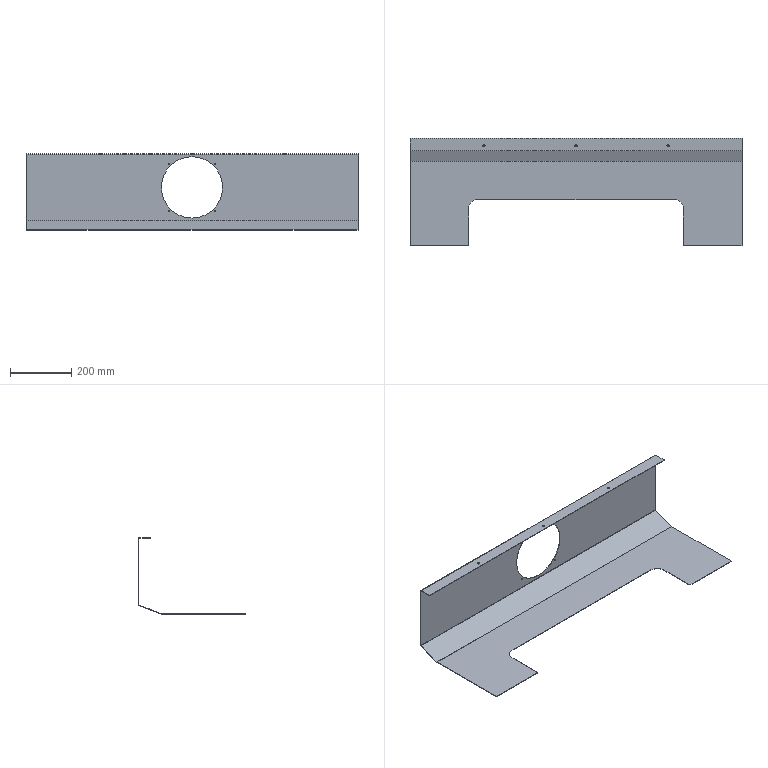Part | SolidWorks | features HoleWzd 2, ICE 2, Fillet 1, FlatPattern 1, SMBaseFlange 1, SheetMetal 1 | 1 solid | 54 faces | box 1082 x 350 x 250 mm | volume 789625 mm3 | plane 28 | cylinder 26 | commonest cylinder face diameters 4 x8 7 x6 0.4 x3 3.4 x3 10 x2 60 x2
STEP:
#1=CARTESIAN_POINT('',(-76.014,348.5,61.986));
#2=VERTEX_POINT('',#1);
#3=CARTESIAN_POINT('',(-76.014,348.5,65.986));
#4=VERTEX_POINT('',#3);
#5=CARTESIAN_POINT('',(-76.014,348.5,63.986));
#6=DIRECTION('',(0.,1.,0.));
#7=DIRECTION('',(0.,0.,1.));
#8=AXIS2_PLACEMENT_3D('',#5,#6,#7);
#9=CIRCLE('',#8,2.);
#10=EDGE_CURVE('',#2,#4,#9,.T.);
#11=ORIENTED_EDGE('',*,*,#10,.F.);
#12=CARTESIAN_POINT('',(-76.014,350.,61.986));
#13=VERTEX_POINT('',#12);
#14=CARTESIAN_POINT('',(-76.014,350.,61.986));
#15=DIRECTION('',(0.,1.,0.));
#16=VECTOR('',#15,1000.);
#17=LINE('',#14,#16);
#18=EDGE_CURVE('',#2,#13,#17,.T.);
#19=ORIENTED_EDGE('',*,*,#18,.T.);
#20=CARTESIAN_POINT('',(-76.014,350.,65.986));
#21=VERTEX_POINT('',#20);
#22=CARTESIAN_POINT('',(-76.014,350.,63.986));
#23=DIRECTION('',(0.,1.,0.));
#24=DIRECTION('',(0.,0.,1.));
#25=AXIS2_PLACEMENT_3D('',#22,#23,#24);
#26=CIRCLE('',#25,2.);
#27=EDGE_CURVE('',#13,#21,#26,.T.);
#28=ORIENTED_EDGE('',*,*,#27,.T.);
#29=CARTESIAN_POINT('',(-76.014,350.,65.986));
#30=DIRECTION('',(0.,1.,0.));
#31=VECTOR('',#30,1000.);
#32=LINE('',#29,#31);
#33=EDGE_CURVE('',#4,#21,#32,.T.);
#34=ORIENTED_EDGE('',*,*,#33,.F.);
#35=EDGE_LOOP('',(#11,#19,#28,#34));
#36=FACE_OUTER_BOUND('',#35,.T.);
#37=CARTESIAN_POINT('',(-76.014,350.,63.986));
#38=DIRECTION('',(0.,1.,0.));
#39=DIRECTION('',(0.,0.,1.));
#40=AXIS2_PLACEMENT_3D('',#37,#38,#39);
#41=CYLINDRICAL_SURFACE('',#40,2.);
#42=ADVANCED_FACE('',(#36),#41,.F.);
#43=CARTESIAN_POINT('',(76.014,348.5,61.986));
#44=VERTEX_POINT('',#43);
#45=CARTESIAN_POINT('',(76.014,348.5,65.986));
#46=VERTEX_POINT('',#45);
#47=CARTESIAN_POINT('',(76.014,348.5,63.986));
#48=DIRECTION('',(0.,1.,0.));
#49=DIRECTION('',(0.,0.,1.));
#50=AXIS2_PLACEMENT_3D('',#47,#48,#49);
#51=CIRCLE('',#50,2.);
#52=EDGE_CURVE('',#44,#46,#51,.T.);
#53=ORIENTED_EDGE('',*,*,#52,.F.);
#54=CARTESIAN_POINT('',(76.014,350.,61.986));
#55=VERTEX_POINT('',#54);
#56=CARTESIAN_POINT('',(76.014,350.,61.986));
#57=DIRECTION('',(0.,1.,0.));
#58=VECTOR('',#57,1000.);
#59=LINE('',#56,#58);
#60=EDGE_CURVE('',#44,#55,#59,.T.);
#61=ORIENTED_EDGE('',*,*,#60,.T.);
#62=CARTESIAN_POINT('',(76.014,350.,65.986));
#63=VERTEX_POINT('',#62);
#64=CARTESIAN_POINT('',(76.014,350.,63.986));
#65=DIRECTION('',(0.,1.,0.));
#66=DIRECTION('',(0.,0.,1.));
#67=AXIS2_PLACEMENT_3D('',#64,#65,#66);
#68=CIRCLE('',#67,2.);
#69=EDGE_CURVE('',#55,#63,#68,.T.);
#70=ORIENTED_EDGE('',*,*,#69,.T.);
#71=CARTESIAN_POINT('',(76.014,350.,65.986));
#72=DIRECTION('',(0.,1.,0.));
#73=VECTOR('',#72,1000.);
#74=LINE('',#71,#73);
#75=EDGE_CURVE('',#46,#63,#74,.T.);
#76=ORIENTED_EDGE('',*,*,#75,.F.);
#77=EDGE_LOOP('',(#53,#61,#70,#76));
#78=FACE_OUTER_BOUND('',#77,.T.);
#79=CARTESIAN_POINT('',(76.014,350.,63.986));
#80=DIRECTION('',(0.,1.,0.));
#81=DIRECTION('',(0.,0.,1.));
#82=AXIS2_PLACEMENT_3D('',#79,#80,#81);
#83=CYLINDRICAL_SURFACE('',#82,2.);
#84=ADVANCED_FACE('',(#78),#83,.F.);
#85=CARTESIAN_POINT('',(76.014,348.5,214.014));
#86=VERTEX_POINT('',#85);
#87=CARTESIAN_POINT('',(76.014,348.5,218.014));
#88=VERTEX_POINT('',#87);
#89=CARTESIAN_POINT('',(76.014,348.5,216.014));
#90=DIRECTION('',(0.,1.,0.));
#91=DIRECTION('',(0.,0.,1.));
#92=AXIS2_PLACEMENT_3D('',#89,#90,#91);
#93=CIRCLE('',#92,2.);
#94=EDGE_CURVE('',#86,#88,#93,.T.);
#95=ORIENTED_EDGE('',*,*,#94,.F.);
#96=CARTESIAN_POINT('',(76.014,350.,214.014));
#97=VERTEX_POINT('',#96);
#98=CARTESIAN_POINT('',(76.014,350.,214.014));
#99=DIRECTION('',(0.,1.,0.));
#100=VECTOR('',#99,1000.);
#101=LINE('',#98,#100);
#102=EDGE_CURVE('',#86,#97,#101,.T.);
#103=ORIENTED_EDGE('',*,*,#102,.T.);
#104=CARTESIAN_POINT('',(76.014,350.,218.014));
#105=VERTEX_POINT('',#104);
#106=CARTESIAN_POINT('',(76.014,350.,216.014));
#107=DIRECTION('',(0.,1.,0.));
#108=DIRECTION('',(0.,0.,1.));
#109=AXIS2_PLACEMENT_3D('',#106,#107,#108);
#110=CIRCLE('',#109,2.);
#111=EDGE_CURVE('',#97,#105,#110,.T.);
#112=ORIENTED_EDGE('',*,*,#111,.T.);
#113=CARTESIAN_POINT('',(76.014,350.,218.014));
#114=DIRECTION('',(0.,1.,0.));
#115=VECTOR('',#114,1000.);
#116=LINE('',#113,#115);
#117=EDGE_CURVE('',#88,#105,#116,.T.);
#118=ORIENTED_EDGE('',*,*,#117,.F.);
#119=EDGE_LOOP('',(#95,#103,#112,#118));
#120=FACE_OUTER_BOUND('',#119,.T.);
#121=CARTESIAN_POINT('',(76.014,350.,216.014));
#122=DIRECTION('',(0.,1.,0.));
#123=DIRECTION('',(0.,0.,1.));
#124=AXIS2_PLACEMENT_3D('',#121,#122,#123);
#125=CYLINDRICAL_SURFACE('',#124,2.);
#126=ADVANCED_FACE('',(#120),#125,.F.);
#127=CARTESIAN_POINT('',(-76.014,348.5,214.014));
#128=VERTEX_POINT('',#127);
#129=CARTESIAN_POINT('',(-76.014,348.5,218.014));
#130=VERTEX_POINT('',#129);
#131=CARTESIAN_POINT('',(-76.014,348.5,216.014));
#132=DIRECTION('',(0.,1.,0.));
#133=DIRECTION('',(0.,0.,1.));
#134=AXIS2_PLACEMENT_3D('',#131,#132,#133);
#135=CIRCLE('',#134,2.);
#136=EDGE_CURVE('',#128,#130,#135,.T.);
#137=ORIENTED_EDGE('',*,*,#136,.F.);
#138=CARTESIAN_POINT('',(-76.014,350.,214.014));
#139=VERTEX_POINT('',#138);
#140=CARTESIAN_POINT('',(-76.014,350.,214.014));
#141=DIRECTION('',(0.,1.,0.));
#142=VECTOR('',#141,1000.);
#143=LINE('',#140,#142);
#144=EDGE_CURVE('',#128,#139,#143,.T.);
#145=ORIENTED_EDGE('',*,*,#144,.T.);
#146=CARTESIAN_POINT('',(-76.014,350.,218.014));
#147=VERTEX_POINT('',#146);
#148=CARTESIAN_POINT('',(-76.014,350.,216.014));
#149=DIRECTION('',(0.,1.,0.));
#150=DIRECTION('',(0.,0.,1.));
#151=AXIS2_PLACEMENT_3D('',#148,#149,#150);
#152=CIRCLE('',#151,2.);
#153=EDGE_CURVE('',#139,#147,#152,.T.);
#154=ORIENTED_EDGE('',*,*,#153,.T.);
#155=CARTESIAN_POINT('',(-76.014,350.,218.014));
#156=DIRECTION('',(0.,1.,0.));
#157=VECTOR('',#156,1000.);
#158=LINE('',#155,#157);
#159=EDGE_CURVE('',#130,#147,#158,.T.);
#160=ORIENTED_EDGE('',*,*,#159,.F.);
#161=EDGE_LOOP('',(#137,#145,#154,#160));
#162=FACE_OUTER_BOUND('',#161,.T.);
#163=CARTESIAN_POINT('',(-76.014,350.,216.014));
#164=DIRECTION('',(0.,1.,0.));
#165=DIRECTION('',(0.,0.,1.));
#166=AXIS2_PLACEMENT_3D('',#163,#164,#165);
#167=CYLINDRICAL_SURFACE('',#166,2.);
#168=ADVANCED_FACE('',(#162),#167,.F.);
#169=CARTESIAN_POINT('',(0.,348.5,240.));
#170=VERTEX_POINT('',#169);
#171=CARTESIAN_POINT('',(0.,348.5,40.));
#172=VERTEX_POINT('',#171);
#173=CARTESIAN_POINT('',(0.,348.5,140.));
#174=DIRECTION('',(0.,-1.,0.));
#175=DIRECTION('',(0.,0.,1.));
#176=AXIS2_PLACEMENT_3D('',#173,#174,#175);
#177=CIRCLE('',#176,100.);
#178=EDGE_CURVE('',#170,#172,#177,.T.);
#179=ORIENTED_EDGE('',*,*,#178,.T.);
#180=CARTESIAN_POINT('',(0.,350.,40.));
#181=VERTEX_POINT('',#180);
#182=CARTESIAN_POINT('',(0.,-0.001,40.));
#183=DIRECTION('',(0.,1.,0.));
#184=VECTOR('',#183,1000.);
#185=LINE('',#182,#184);
#186=EDGE_CURVE('',#172,#181,#185,.T.);
#187=ORIENTED_EDGE('',*,*,#186,.T.);
#188=CARTESIAN_POINT('',(0.,350.,240.));
#189=VERTEX_POINT('',#188);
#190=CARTESIAN_POINT('',(0.,350.,140.));
#191=DIRECTION('',(0.,1.,0.));
#192=DIRECTION('',(0.,0.,1.));
#193=AXIS2_PLACEMENT_3D('',#190,#191,#192);
#194=CIRCLE('',#193,100.);
#195=EDGE_CURVE('',#181,#189,#194,.T.);
#196=ORIENTED_EDGE('',*,*,#195,.T.);
#197=CARTESIAN_POINT('',(0.,-0.001,240.));
#198=DIRECTION('',(0.,1.,0.));
#199=VECTOR('',#198,1000.);
#200=LINE('',#197,#199);
#201=EDGE_CURVE('',#170,#189,#200,.T.);
#202=ORIENTED_EDGE('',*,*,#201,.F.);
#203=EDGE_LOOP('',(#179,#187,#196,#202));
#204=FACE_OUTER_BOUND('',#203,.T.);
#205=CARTESIAN_POINT('',(0.,-0.001,140.));
#206=DIRECTION('',(0.,1.,0.));
#207=DIRECTION('',(0.,0.,1.));
#208=AXIS2_PLACEMENT_3D('',#205,#206,#207);
#209=CYLINDRICAL_SURFACE('',#208,100.);
#210=ADVANCED_FACE('',(#204),#209,.F.);
#211=CARTESIAN_POINT('',(-303.5,325.,248.5));
#212=VERTEX_POINT('',#211);
#213=CARTESIAN_POINT('',(-296.5,325.,248.5));
#214=VERTEX_POINT('',#213);
#215=CARTESIAN_POINT('',(-300.,325.,248.5));
#216=DIRECTION('',(0.,0.,1.));
#217=DIRECTION('',(1.,0.,0.));
#218=AXIS2_PLACEMENT_3D('',#215,#216,#217);
#219=CIRCLE('',#218,3.5);
#220=EDGE_CURVE('',#212,#214,#219,.T.);
#221=ORIENTED_EDGE('',*,*,#220,.F.);
#222=CARTESIAN_POINT('',(-303.5,325.,250.));
#223=VERTEX_POINT('',#222);
#224=CARTESIAN_POINT('',(-303.5,325.,250.));
#225=DIRECTION('',(0.,0.,1.));
#226=VECTOR('',#225,1000.);
#227=LINE('',#224,#226);
#228=EDGE_CURVE('',#212,#223,#227,.T.);
#229=ORIENTED_EDGE('',*,*,#228,.T.);
#230=CARTESIAN_POINT('',(-296.5,325.,250.));
#231=VERTEX_POINT('',#230);
#232=CARTESIAN_POINT('',(-300.,325.,250.));
#233=DIRECTION('',(0.,0.,1.));
#234=DIRECTION('',(1.,0.,0.));
#235=AXIS2_PLACEMENT_3D('',#232,#233,#234);
#236=CIRCLE('',#235,3.5);
#237=EDGE_CURVE('',#223,#231,#236,.T.);
#238=ORIENTED_EDGE('',*,*,#237,.T.);
#239=CARTESIAN_POINT('',(-296.5,325.,250.));
#240=DIRECTION('',(0.,0.,1.));
#241=VECTOR('',#240,1000.);
#242=LINE('',#239,#241);
#243=EDGE_CURVE('',#214,#231,#242,.T.);
#244=ORIENTED_EDGE('',*,*,#243,.F.);
#245=EDGE_LOOP('',(#221,#229,#238,#244));
#246=FACE_OUTER_BOUND('',#245,.T.);
#247=CARTESIAN_POINT('',(-300.,325.,250.));
#248=DIRECTION('',(0.,0.,1.));
#249=DIRECTION('',(1.,0.,0.));
#250=AXIS2_PLACEMENT_3D('',#247,#248,#249);
#251=CYLINDRICAL_SURFACE('',#250,3.5);
#252=ADVANCED_FACE('',(#246),#251,.F.);
#253=CARTESIAN_POINT('',(-3.5,325.,248.5));
#254=VERTEX_POINT('',#253);
#255=CARTESIAN_POINT('',(3.5,325.,248.5));
#256=VERTEX_POINT('',#255);
#257=CARTESIAN_POINT('',(0.,325.,248.5));
#258=DIRECTION('',(0.,0.,1.));
#259=DIRECTION('',(1.,0.,0.));
#260=AXIS2_PLACEMENT_3D('',#257,#258,#259);
#261=CIRCLE('',#260,3.5);
#262=EDGE_CURVE('',#254,#256,#261,.T.);
#263=ORIENTED_EDGE('',*,*,#262,.F.);
#264=CARTESIAN_POINT('',(-3.5,325.,250.));
#265=VERTEX_POINT('',#264);
#266=CARTESIAN_POINT('',(-3.5,325.,250.));
#267=DIRECTION('',(0.,0.,1.));
#268=VECTOR('',#267,1000.);
#269=LINE('',#266,#268);
#270=EDGE_CURVE('',#254,#265,#269,.T.);
#271=ORIENTED_EDGE('',*,*,#270,.T.);
#272=CARTESIAN_POINT('',(3.5,325.,250.));
#273=VERTEX_POINT('',#272);
#274=CARTESIAN_POINT('',(0.,325.,250.));
#275=DIRECTION('',(0.,0.,1.));
#276=DIRECTION('',(1.,0.,0.));
#277=AXIS2_PLACEMENT_3D('',#274,#275,#276);
#278=CIRCLE('',#277,3.5);
#279=EDGE_CURVE('',#265,#273,#278,.T.);
#280=ORIENTED_EDGE('',*,*,#279,.T.);
#281=CARTESIAN_POINT('',(3.5,325.,250.));
#282=DIRECTION('',(0.,0.,1.));
#283=VECTOR('',#282,1000.);
#284=LINE('',#281,#283);
#285=EDGE_CURVE('',#256,#273,#284,.T.);
#286=ORIENTED_EDGE('',*,*,#285,.F.);
#287=EDGE_LOOP('',(#263,#271,#280,#286));
#288=FACE_OUTER_BOUND('',#287,.T.);
#289=CARTESIAN_POINT('',(0.,325.,250.));
#290=DIRECTION('',(0.,0.,1.));
#291=DIRECTION('',(1.,0.,0.));
#292=AXIS2_PLACEMENT_3D('',#289,#290,#291);
#293=CYLINDRICAL_SURFACE('',#292,3.5);
#294=ADVANCED_FACE('',(#288),#293,.F.);
#295=CARTESIAN_POINT('',(296.5,325.,248.5));
#296=VERTEX_POINT('',#295);
#297=CARTESIAN_POINT('',(303.5,325.,248.5));
#298=VERTEX_POINT('',#297);
#299=CARTESIAN_POINT('',(300.,325.,248.5));
#300=DIRECTION('',(0.,0.,1.));
#301=DIRECTION('',(1.,0.,0.));
#302=AXIS2_PLACEMENT_3D('',#299,#300,#301);
#303=CIRCLE('',#302,3.5);
#304=EDGE_CURVE('',#296,#298,#303,.T.);
#305=ORIENTED_EDGE('',*,*,#304,.F.);
#306=CARTESIAN_POINT('',(296.5,325.,250.));
#307=VERTEX_POINT('',#306);
#308=CARTESIAN_POINT('',(296.5,325.,250.));
#309=DIRECTION('',(0.,0.,1.));
#310=VECTOR('',#309,1000.);
#311=LINE('',#308,#310);
#312=EDGE_CURVE('',#296,#307,#311,.T.);
#313=ORIENTED_EDGE('',*,*,#312,.T.);
#314=CARTESIAN_POINT('',(303.5,325.,250.));
#315=VERTEX_POINT('',#314);
#316=CARTESIAN_POINT('',(300.,325.,250.));
#317=DIRECTION('',(0.,0.,1.));
#318=DIRECTION('',(1.,0.,0.));
#319=AXIS2_PLACEMENT_3D('',#316,#317,#318);
#320=CIRCLE('',#319,3.5);
#321=EDGE_CURVE('',#307,#315,#320,.T.);
#322=ORIENTED_EDGE('',*,*,#321,.T.);
#323=CARTESIAN_POINT('',(303.5,325.,250.));
#324=DIRECTION('',(0.,0.,1.));
#325=VECTOR('',#324,1000.);
#326=LINE('',#323,#325);
#327=EDGE_CURVE('',#298,#315,#326,.T.);
#328=ORIENTED_EDGE('',*,*,#327,.F.);
#329=EDGE_LOOP('',(#305,#313,#322,#328));
#330=FACE_OUTER_BOUND('',#329,.T.);
#331=CARTESIAN_POINT('',(300.,325.,250.));
#332=DIRECTION('',(0.,0.,1.));
#333=DIRECTION('',(1.,0.,0.));
#334=AXIS2_PLACEMENT_3D('',#331,#332,#333);
#335=CYLINDRICAL_SURFACE('',#334,3.5);
#336=ADVANCED_FACE('',(#330),#335,.F.);
#337=CARTESIAN_POINT('',(541.,0.,1.5));
#338=VERTEX_POINT('',#337);
#339=CARTESIAN_POINT('',(355.,0.,1.5));
#340=VERTEX_POINT('',#339);
#341=CARTESIAN_POINT('',(541.,0.,1.5));
#342=DIRECTION('',(-1.,0.,0.));
#343=VECTOR('',#342,1000.);
#344=LINE('',#341,#343);
#345=EDGE_CURVE('',#338,#340,#344,.T.);
#346=ORIENTED_EDGE('',*,*,#345,.T.);
#347=CARTESIAN_POINT('',(355.,0.,0.));
#348=VERTEX_POINT('',#347);
#349=CARTESIAN_POINT('',(355.,0.,0.));
#350=DIRECTION('',(0.,0.,-1.));
#351=VECTOR('',#350,1000.);
#352=LINE('',#349,#351);
#353=EDGE_CURVE('',#340,#348,#352,.T.);
#354=ORIENTED_EDGE('',*,*,#353,.T.);
#355=CARTESIAN_POINT('',(541.,0.,0.));
#356=VERTEX_POINT('',#355);
#357=CARTESIAN_POINT('',(541.,0.,0.));
#358=DIRECTION('',(-1.,0.,0.));
#359=VECTOR('',#358,1000.);
#360=LINE('',#357,#359);
#361=EDGE_CURVE('',#356,#348,#360,.T.);
#362=ORIENTED_EDGE('',*,*,#361,.F.);
#363=CARTESIAN_POINT('',(541.,0.,0.));
#364=DIRECTION('',(0.,0.,1.));
#365=VECTOR('',#364,1000.);
#366=LINE('',#363,#365);
#367=EDGE_CURVE('',#356,#338,#366,.T.);
#368=ORIENTED_EDGE('',*,*,#367,.T.);
#369=EDGE_LOOP('',(#346,#354,#362,#368));
#370=FACE_OUTER_BOUND('',#369,.T.);
#371=CARTESIAN_POINT('',(541.,0.,0.));
#372=DIRECTION('',(0.,-1.,0.));
#373=DIRECTION('',(0.,0.,-1.));
#374=AXIS2_PLACEMENT_3D('',#371,#372,#373);
#375=PLANE('',#374);
#376=ADVANCED_FACE('',(#370),#375,.T.);
#377=CARTESIAN_POINT('',(541.,350.,248.3));
#378=VERTEX_POINT('',#377);
#379=CARTESIAN_POINT('',(541.,348.5,248.3));
#380=VERTEX_POINT('',#379);
#381=CARTESIAN_POINT('',(541.,350.,248.3));
#382=DIRECTION('',(0.,-1.,0.));
#383=VECTOR('',#382,1000.);
#384=LINE('',#381,#383);
#385=EDGE_CURVE('',#378,#380,#384,.T.);
#386=ORIENTED_EDGE('',*,*,#385,.F.);
#387=CARTESIAN_POINT('',(541.,348.3,250.));
#388=VERTEX_POINT('',#387);
#389=CARTESIAN_POINT('',(541.,348.3,248.3));
#390=DIRECTION('',(-1.,0.,0.));
#391=DIRECTION('',(0.,0.,-1.));
#392=AXIS2_PLACEMENT_3D('',#389,#390,#391);
#393=CIRCLE('',#392,1.7);
#394=EDGE_CURVE('',#388,#378,#393,.T.);
#395=ORIENTED_EDGE('',*,*,#394,.F.);
#396=CARTESIAN_POINT('',(541.,348.3,248.5));
#397=VERTEX_POINT('',#396);
#398=CARTESIAN_POINT('',(541.,348.3,248.5));
#399=DIRECTION('',(0.,0.,1.));
#400=VECTOR('',#399,1000.);
#401=LINE('',#398,#400);
#402=EDGE_CURVE('',#397,#388,#401,.T.);
#403=ORIENTED_EDGE('',*,*,#402,.F.);
#404=CARTESIAN_POINT('',(541.,348.3,248.3));
#405=DIRECTION('',(-1.,0.,0.));
#406=DIRECTION('',(0.,0.,-1.));
#407=AXIS2_PLACEMENT_3D('',#404,#405,#406);
#408=CIRCLE('',#407,0.2);
#409=EDGE_CURVE('',#397,#380,#408,.T.);
#410=ORIENTED_EDGE('',*,*,#409,.T.);
#411=EDGE_LOOP('',(#386,#395,#403,#410));
#412=FACE_OUTER_BOUND('',#411,.T.);
#413=CARTESIAN_POINT('',(541.,350.,248.3));
#414=DIRECTION('',(1.,0.,0.));
#415=DIRECTION('',(0.,0.,-1.));
#416=AXIS2_PLACEMENT_3D('',#413,#414,#415);
#417=PLANE('',#416);
#418=ADVANCED_FACE('',(#412),#417,.T.);
#419=CARTESIAN_POINT('',(541.,350.,31.151));
#420=VERTEX_POINT('',#419);
#421=CARTESIAN_POINT('',(541.,350.,250.));
#422=DIRECTION('',(0.,0.,-1.));
#423=VECTOR('',#422,1000.);
#424=LINE('',#421,#423);
#425=EDGE_CURVE('',#378,#420,#424,.T.);
#426=ORIENTED_EDGE('',*,*,#425,.F.);
#427=ORIENTED_EDGE('',*,*,#385,.T.);
#428=CARTESIAN_POINT('',(541.,348.5,31.151));
#429=VERTEX_POINT('',#428);
#430=CARTESIAN_POINT('',(541.,348.5,250.));
#431=DIRECTION('',(0.,0.,-1.));
#432=VECTOR('',#431,1000.);
#433=LINE('',#430,#432);
#434=EDGE_CURVE('',#380,#429,#433,.T.);
#435=ORIENTED_EDGE('',*,*,#434,.T.);
#436=CARTESIAN_POINT('',(541.,348.5,31.151));
#437=DIRECTION('',(0.,1.,0.));
#438=VECTOR('',#437,1000.);
#439=LINE('',#436,#438);
#440=EDGE_CURVE('',#429,#420,#439,.T.);
#441=ORIENTED_EDGE('',*,*,#440,.T.);
#442=EDGE_LOOP('',(#426,#427,#435,#441));
#443=FACE_OUTER_BOUND('',#442,.T.);
#444=CARTESIAN_POINT('',(541.,348.3,248.5));
#445=DIRECTION('',(1.,0.,0.));
#446=DIRECTION('',(0.,0.,-1.));
#447=AXIS2_PLACEMENT_3D('',#444,#445,#446);
#448=PLANE('',#447);
#449=ADVANCED_FACE('',(#443),#448,.T.);
#450=CARTESIAN_POINT('',(-541.,348.3,250.));
#451=VERTEX_POINT('',#450);
#452=CARTESIAN_POINT('',(-541.,348.3,248.5));
#453=VERTEX_POINT('',#452);
#454=CARTESIAN_POINT('',(-541.,348.3,250.));
#455=DIRECTION('',(0.,0.,-1.));
#456=VECTOR('',#455,1000.);
#457=LINE('',#454,#456);
#458=EDGE_CURVE('',#451,#453,#457,.T.);
#459=ORIENTED_EDGE('',*,*,#458,.F.);
#460=CARTESIAN_POINT('',(-541.,350.,248.3));
#461=VERTEX_POINT('',#460);
#462=CARTESIAN_POINT('',(-541.,348.3,248.3));
#463=DIRECTION('',(-1.,0.,0.));
#464=DIRECTION('',(0.,0.,-1.));
#465=AXIS2_PLACEMENT_3D('',#462,#463,#464);
#466=CIRCLE('',#465,1.7);
#467=EDGE_CURVE('',#451,#461,#466,.T.);
#468=ORIENTED_EDGE('',*,*,#467,.T.);
#469=CARTESIAN_POINT('',(-541.,348.5,248.3));
#470=VERTEX_POINT('',#469);
#471=CARTESIAN_POINT('',(-541.,348.5,248.3));
#472=DIRECTION('',(0.,1.,0.));
#473=VECTOR('',#472,1000.);
#474=LINE('',#471,#473);
#475=EDGE_CURVE('',#470,#461,#474,.T.);
#476=ORIENTED_EDGE('',*,*,#475,.F.);
#477=CARTESIAN_POINT('',(-541.,348.3,248.3));
#478=DIRECTION('',(-1.,0.,0.));
#479=DIRECTION('',(0.,0.,-1.));
#480=AXIS2_PLACEMENT_3D('',#477,#478,#479);
#481=CIRCLE('',#480,0.2);
#482=EDGE_CURVE('',#453,#470,#481,.T.);
#483=ORIENTED_EDGE('',*,*,#482,.F.);
#484=EDGE_LOOP('',(#459,#468,#476,#483));
#485=FACE_OUTER_BOUND('',#484,.T.);
#486=CARTESIAN_POINT('',(-541.,348.3,250.));
#487=DIRECTION('',(-1.,0.,0.));
#488=DIRECTION('',(0.,0.,1.));
#489=AXIS2_PLACEMENT_3D('',#486,#487,#488);
#490=PLANE('',#489);
#491=ADVANCED_FACE('',(#485),#490,.T.);
#492=CARTESIAN_POINT('',(-541.,310.,250.));
#493=VERTEX_POINT('',#492);
#494=CARTESIAN_POINT('',(-541.,310.,250.));
#495=DIRECTION('',(0.,1.,0.));
#496=VECTOR('',#495,1000.);
#497=LINE('',#494,#496);
#498=EDGE_CURVE('',#493,#451,#497,.T.);
#499=ORIENTED_EDGE('',*,*,#498,.T.);
#500=ORIENTED_EDGE('',*,*,#458,.T.);
#501=CARTESIAN_POINT('',(-541.,310.,248.5));
#502=VERTEX_POINT('',#501);
#503=CARTESIAN_POINT('',(-541.,310.,248.5));
#504=DIRECTION('',(0.,1.,0.));
#505=VECTOR('',#504,1000.);
#506=LINE('',#503,#505);
#507=EDGE_CURVE('',#502,#453,#506,.T.);
#508=ORIENTED_EDGE('',*,*,#507,.F.);
#509=CARTESIAN_POINT('',(-541.,310.,248.5));
#510=DIRECTION('',(0.,0.,1.));
#511=VECTOR('',#510,1000.);
#512=LINE('',#509,#511);
#513=EDGE_CURVE('',#502,#493,#512,.T.);
#514=ORIENTED_EDGE('',*,*,#513,.T.);
#515=EDGE_LOOP('',(#499,#500,#508,#514));
#516=FACE_OUTER_BOUND('',#515,.T.);
#517=CARTESIAN_POINT('',(-541.,348.5,248.3));
#518=DIRECTION('',(-1.,0.,0.));
#519=DIRECTION('',(0.,0.,1.));
#520=AXIS2_PLACEMENT_3D('',#517,#518,#519);
#521=PLANE('',#520);
#522=ADVANCED_FACE('',(#516),#521,.T.);
#523=CARTESIAN_POINT('',(541.,348.931,29.573));
#524=VERTEX_POINT('',#523);
#525=CARTESIAN_POINT('',(541.,348.374,30.965));
#526=VERTEX_POINT('',#525);
#527=CARTESIAN_POINT('',(541.,348.931,29.573));
#528=DIRECTION('',(0.,-0.3714,0.9285));
#529=VECTOR('',#528,1000.);
#530=LINE('',#527,#529);
#531=EDGE_CURVE('',#524,#526,#530,.T.);
#532=ORIENTED_EDGE('',*,*,#531,.F.);
#533=CARTESIAN_POINT('',(541.,348.3,31.151));
#534=DIRECTION('',(-1.,0.,0.));
#535=DIRECTION('',(0.,0.,-1.));
#536=AXIS2_PLACEMENT_3D('',#533,#534,#535);
#537=CIRCLE('',#536,1.7);
#538=EDGE_CURVE('',#420,#524,#537,.T.);
#539=ORIENTED_EDGE('',*,*,#538,.F.);
#540=ORIENTED_EDGE('',*,*,#440,.F.);
#541=CARTESIAN_POINT('',(541.,348.3,31.151));
#542=DIRECTION('',(-1.,0.,0.));
#543=DIRECTION('',(0.,0.,-1.));
#544=AXIS2_PLACEMENT_3D('',#541,#542,#543);
#545=CIRCLE('',#544,0.2);
#546=EDGE_CURVE('',#429,#526,#545,.T.);
#547=ORIENTED_EDGE('',*,*,#546,.T.);
#548=EDGE_LOOP('',(#532,#539,#540,#547));
#549=FACE_OUTER_BOUND('',#548,.T.);
#550=CARTESIAN_POINT('',(541.,348.931,29.573));
#551=DIRECTION('',(1.,0.,0.));
#552=DIRECTION('',(0.,0.,-1.));
#553=AXIS2_PLACEMENT_3D('',#550,#551,#552);
#554=PLANE('',#553);
#555=ADVANCED_FACE('',(#549),#554,.T.);
#556=CARTESIAN_POINT('',(541.,275.304,0.1216));
#557=VERTEX_POINT('',#556);
#558=CARTESIAN_POINT('',(541.,350.,30.));
#559=DIRECTION('',(0.,-0.9285,-0.3714));
#560=VECTOR('',#559,1000.);
#561=LINE('',#558,#560);
#562=EDGE_CURVE('',#524,#557,#561,.T.);
#563=ORIENTED_EDGE('',*,*,#562,.F.);
#564=ORIENTED_EDGE('',*,*,#531,.T.);
#565=CARTESIAN_POINT('',(541.,274.747,1.514));
#566=VERTEX_POINT('',#565);
#567=CARTESIAN_POINT('',(541.,349.443,31.393));
#568=DIRECTION('',(0.,-0.9285,-0.3714));
#569=VECTOR('',#568,1000.);
#570=LINE('',#567,#569);
#571=EDGE_CURVE('',#526,#566,#570,.T.);
#572=ORIENTED_EDGE('',*,*,#571,.T.);
#573=CARTESIAN_POINT('',(541.,274.747,1.514));
#574=DIRECTION('',(0.,0.3714,-0.9285));
#575=VECTOR('',#574,1000.);
#576=LINE('',#573,#575);
#577=EDGE_CURVE('',#566,#557,#576,.T.);
#578=ORIENTED_EDGE('',*,*,#577,.T.);
#579=EDGE_LOOP('',(#563,#564,#572,#578));
#580=FACE_OUTER_BOUND('',#579,.T.);
#581=CARTESIAN_POINT('',(541.,348.5,31.151));
#582=DIRECTION('',(1.,0.,0.));
#583=DIRECTION('',(0.,0.,-1.));
#584=AXIS2_PLACEMENT_3D('',#581,#582,#583);
#585=PLANE('',#584);
#586=ADVANCED_FACE('',(#580),#585,.T.);
#587=CARTESIAN_POINT('',(-541.,350.,31.151));
#588=VERTEX_POINT('',#587);
#589=CARTESIAN_POINT('',(-541.,348.5,31.151));
#590=VERTEX_POINT('',#589);
#591=CARTESIAN_POINT('',(-541.,350.,31.151));
#592=DIRECTION('',(0.,-1.,0.));
#593=VECTOR('',#592,1000.);
#594=LINE('',#591,#593);
#595=EDGE_CURVE('',#588,#590,#594,.T.);
#596=ORIENTED_EDGE('',*,*,#595,.F.);
#597=CARTESIAN_POINT('',(-541.,348.931,29.573));
#598=VERTEX_POINT('',#597);
#599=CARTESIAN_POINT('',(-541.,348.3,31.151));
#600=DIRECTION('',(-1.,0.,0.));
#601=DIRECTION('',(0.,0.,-1.));
#602=AXIS2_PLACEMENT_3D('',#599,#600,#601);
#603=CIRCLE('',#602,1.7);
#604=EDGE_CURVE('',#588,#598,#603,.T.);
#605=ORIENTED_EDGE('',*,*,#604,.T.);
#606=CARTESIAN_POINT('',(-541.,348.374,30.965));
#607=VERTEX_POINT('',#606);
#608=CARTESIAN_POINT('',(-541.,348.374,30.965));
#609=DIRECTION('',(0.,0.3714,-0.9285));
#610=VECTOR('',#609,1000.);
#611=LINE('',#608,#610);
#612=EDGE_CURVE('',#607,#598,#611,.T.);
#613=ORIENTED_EDGE('',*,*,#612,.F.);
#614=CARTESIAN_POINT('',(-541.,348.3,31.151));
#615=DIRECTION('',(-1.,0.,0.));
#616=DIRECTION('',(0.,0.,-1.));
#617=AXIS2_PLACEMENT_3D('',#614,#615,#616);
#618=CIRCLE('',#617,0.2);
#619=EDGE_CURVE('',#590,#607,#618,.T.);
#620=ORIENTED_EDGE('',*,*,#619,.F.);
#621=EDGE_LOOP('',(#596,#605,#613,#620));
#622=FACE_OUTER_BOUND('',#621,.T.);
#623=CARTESIAN_POINT('',(-541.,350.,31.151));
#624=DIRECTION('',(-1.,0.,0.));
#625=DIRECTION('',(0.,0.,1.));
#626=AXIS2_PLACEMENT_3D('',#623,#624,#625);
#627=PLANE('',#626);
#628=ADVANCED_FACE('',(#622),#627,.T.);
#629=CARTESIAN_POINT('',(-541.,350.,250.));
#630=DIRECTION('',(0.,0.,-1.));
#631=VECTOR('',#630,1000.);
#632=LINE('',#629,#631);
#633=EDGE_CURVE('',#461,#588,#632,.T.);
#634=ORIENTED_EDGE('',*,*,#633,.T.);
#635=ORIENTED_EDGE('',*,*,#595,.T.);
#636=CARTESIAN_POINT('',(-541.,348.5,250.));
#637=DIRECTION('',(0.,0.,-1.));
#638=VECTOR('',#637,1000.);
#639=LINE('',#636,#638);
#640=EDGE_CURVE('',#470,#590,#639,.T.);
#641=ORIENTED_EDGE('',*,*,#640,.F.);
#642=ORIENTED_EDGE('',*,*,#475,.T.);
#643=EDGE_LOOP('',(#634,#635,#641,#642));
#644=FACE_OUTER_BOUND('',#643,.T.);
#645=CARTESIAN_POINT('',(-541.,348.374,30.965));
#646=DIRECTION('',(-1.,0.,0.));
#647=DIRECTION('',(0.,0.,1.));
#648=AXIS2_PLACEMENT_3D('',#645,#646,#647);
#649=PLANE('',#648);
#650=ADVANCED_FACE('',(#644),#649,.T.);
#651=CARTESIAN_POINT('',(541.,274.673,0.));
#652=VERTEX_POINT('',#651);
#653=CARTESIAN_POINT('',(541.,274.673,1.5));
#654=VERTEX_POINT('',#653);
#655=CARTESIAN_POINT('',(541.,274.673,0.));
#656=DIRECTION('',(0.,0.,1.));
#657=VECTOR('',#656,1000.);
#658=LINE('',#655,#657);
#659=EDGE_CURVE('',#652,#654,#658,.T.);
#660=ORIENTED_EDGE('',*,*,#659,.F.);
#661=CARTESIAN_POINT('',(541.,274.673,1.7));
#662=DIRECTION('',(-1.,0.,0.));
#663=DIRECTION('',(0.,0.,-1.));
#664=AXIS2_PLACEMENT_3D('',#661,#662,#663);
#665=CIRCLE('',#664,1.7);
#666=EDGE_CURVE('',#557,#652,#665,.T.);
#667=ORIENTED_EDGE('',*,*,#666,.F.);
#668=ORIENTED_EDGE('',*,*,#577,.F.);
#669=CARTESIAN_POINT('',(541.,274.673,1.7));
#670=DIRECTION('',(-1.,0.,0.));
#671=DIRECTION('',(0.,0.,-1.));
#672=AXIS2_PLACEMENT_3D('',#669,#670,#671);
#673=CIRCLE('',#672,0.2);
#674=EDGE_CURVE('',#566,#654,#673,.T.);
#675=ORIENTED_EDGE('',*,*,#674,.T.);
#676=EDGE_LOOP('',(#660,#667,#668,#675));
#677=FACE_OUTER_BOUND('',#676,.T.);
#678=CARTESIAN_POINT('',(541.,274.673,0.));
#679=DIRECTION('',(1.,0.,0.));
#680=DIRECTION('',(0.,0.,-1.));
#681=AXIS2_PLACEMENT_3D('',#678,#679,#680);
#682=PLANE('',#681);
#683=ADVANCED_FACE('',(#677),#682,.T.);
#684=CARTESIAN_POINT('',(541.,275.,0.));
#685=DIRECTION('',(0.,-1.,0.));
#686=VECTOR('',#685,1000.);
#687=LINE('',#684,#686);
#688=EDGE_CURVE('',#652,#356,#687,.T.);
#689=ORIENTED_EDGE('',*,*,#688,.F.);
#690=ORIENTED_EDGE('',*,*,#659,.T.);
#691=CARTESIAN_POINT('',(541.,275.,1.5));
#692=DIRECTION('',(0.,-1.,0.));
#693=VECTOR('',#692,1000.);
#694=LINE('',#691,#693);
#695=EDGE_CURVE('',#654,#338,#694,.T.);
#696=ORIENTED_EDGE('',*,*,#695,.T.);
#697=ORIENTED_EDGE('',*,*,#367,.F.);
#698=EDGE_LOOP('',(#689,#690,#696,#697));
#699=FACE_OUTER_BOUND('',#698,.T.);
#700=CARTESIAN_POINT('',(541.,274.747,1.514));
#701=DIRECTION('',(1.,0.,0.));
#702=DIRECTION('',(0.,0.,-1.));
#703=AXIS2_PLACEMENT_3D('',#700,#701,#702);
#704=PLANE('',#703);
#705=ADVANCED_FACE('',(#699),#704,.T.);
#706=CARTESIAN_POINT('',(-541.,275.304,0.1216));
#707=VERTEX_POINT('',#706);
#708=CARTESIAN_POINT('',(-541.,274.747,1.514));
#709=VERTEX_POINT('',#708);
#710=CARTESIAN_POINT('',(-541.,275.304,0.1216));
#711=DIRECTION('',(0.,-0.3714,0.9285));
#712=VECTOR('',#711,1000.);
#713=LINE('',#710,#712);
#714=EDGE_CURVE('',#707,#709,#713,.T.);
#715=ORIENTED_EDGE('',*,*,#714,.F.);
#716=CARTESIAN_POINT('',(-541.,274.673,0.));
#717=VERTEX_POINT('',#716);
#718=CARTESIAN_POINT('',(-541.,274.673,1.7));
#719=DIRECTION('',(-1.,0.,0.));
#720=DIRECTION('',(0.,0.,-1.));
#721=AXIS2_PLACEMENT_3D('',#718,#719,#720);
#722=CIRCLE('',#721,1.7);
#723=EDGE_CURVE('',#707,#717,#722,.T.);
#724=ORIENTED_EDGE('',*,*,#723,.T.);
#725=CARTESIAN_POINT('',(-541.,274.673,1.5));
#726=VERTEX_POINT('',#725);
#727=CARTESIAN_POINT('',(-541.,274.673,1.5));
#728=DIRECTION('',(0.,0.,-1.));
#729=VECTOR('',#728,1000.);
#730=LINE('',#727,#729);
#731=EDGE_CURVE('',#726,#717,#730,.T.);
#732=ORIENTED_EDGE('',*,*,#731,.F.);
#733=CARTESIAN_POINT('',(-541.,274.673,1.7));
#734=DIRECTION('',(-1.,0.,0.));
#735=DIRECTION('',(0.,0.,-1.));
#736=AXIS2_PLACEMENT_3D('',#733,#734,#735);
#737=CIRCLE('',#736,0.2);
#738=EDGE_CURVE('',#709,#726,#737,.T.);
#739=ORIENTED_EDGE('',*,*,#738,.F.);
#740=EDGE_LOOP('',(#715,#724,#732,#739));
#741=FACE_OUTER_BOUND('',#740,.T.);
#742=CARTESIAN_POINT('',(-541.,275.304,0.1216));
#743=DIRECTION('',(-1.,0.,0.));
#744=DIRECTION('',(0.,0.,1.));
#745=AXIS2_PLACEMENT_3D('',#742,#743,#744);
#746=PLANE('',#745);
#747=ADVANCED_FACE('',(#741),#746,.T.);
#748=CARTESIAN_POINT('',(-541.,350.,30.));
#749=DIRECTION('',(0.,-0.9285,-0.3714));
#750=VECTOR('',#749,1000.);
#751=LINE('',#748,#750);
#752=EDGE_CURVE('',#598,#707,#751,.T.);
#753=ORIENTED_EDGE('',*,*,#752,.T.);
#754=ORIENTED_EDGE('',*,*,#714,.T.);
#755=CARTESIAN_POINT('',(-541.,349.443,31.393));
#756=DIRECTION('',(0.,-0.9285,-0.3714));
#757=VECTOR('',#756,1000.);
#758=LINE('',#755,#757);
#759=EDGE_CURVE('',#607,#709,#758,.T.);
#760=ORIENTED_EDGE('',*,*,#759,.F.);
#761=ORIENTED_EDGE('',*,*,#612,.T.);
#762=EDGE_LOOP('',(#753,#754,#760,#761));
#763=FACE_OUTER_BOUND('',#762,.T.);
#764=CARTESIAN_POINT('',(-541.,274.673,1.5));
#765=DIRECTION('',(-1.,0.,0.));
#766=DIRECTION('',(0.,0.,1.));
#767=AXIS2_PLACEMENT_3D('',#764,#765,#766);
#768=PLANE('',#767);
#769=ADVANCED_FACE('',(#763),#768,.T.);
#770=CARTESIAN_POINT('',(-355.,0.,1.5));
#771=VERTEX_POINT('',#770);
#772=CARTESIAN_POINT('',(-541.,0.,1.5));
#773=VERTEX_POINT('',#772);
#774=CARTESIAN_POINT('',(541.,0.,1.5));
#775=DIRECTION('',(-1.,0.,0.));
#776=VECTOR('',#775,1000.);
#777=LINE('',#774,#776);
#778=EDGE_CURVE('',#771,#773,#777,.T.);
#779=ORIENTED_EDGE('',*,*,#778,.F.);
#780=CARTESIAN_POINT('',(-350.,5.,1.5));
#781=VERTEX_POINT('',#780);
#782=CARTESIAN_POINT('',(-355.,5.,1.5));
#783=DIRECTION('',(0.,0.,1.));
#784=DIRECTION('',(-1.,0.,0.));
#785=AXIS2_PLACEMENT_3D('',#782,#783,#784);
#786=CIRCLE('',#785,5.);
#787=EDGE_CURVE('',#771,#781,#786,.T.);
#788=ORIENTED_EDGE('',*,*,#787,.T.);
#789=CARTESIAN_POINT('',(-350.,120.,1.5));
#790=VERTEX_POINT('',#789);
#791=CARTESIAN_POINT('',(-350.,275.,1.5));
#792=DIRECTION('',(0.,1.,0.));
#793=VECTOR('',#792,1000.);
#794=LINE('',#791,#793);
#795=EDGE_CURVE('',#781,#790,#794,.T.);
#796=ORIENTED_EDGE('',*,*,#795,.T.);
#797=CARTESIAN_POINT('',(-320.,150.,1.5));
#798=VERTEX_POINT('',#797);
#799=CARTESIAN_POINT('',(-320.,120.,1.5));
#800=DIRECTION('',(0.,0.,-1.));
#801=DIRECTION('',(-1.,0.,0.));
#802=AXIS2_PLACEMENT_3D('',#799,#800,#801);
#803=CIRCLE('',#802,30.);
#804=EDGE_CURVE('',#790,#798,#803,.T.);
#805=ORIENTED_EDGE('',*,*,#804,.T.);
#806=CARTESIAN_POINT('',(320.,150.,1.5));
#807=VERTEX_POINT('',#806);
#808=CARTESIAN_POINT('',(541.,150.,1.5));
#809=DIRECTION('',(1.,0.,0.));
#810=VECTOR('',#809,1000.);
#811=LINE('',#808,#810);
#812=EDGE_CURVE('',#798,#807,#811,.T.);
#813=ORIENTED_EDGE('',*,*,#812,.T.);
#814=CARTESIAN_POINT('',(350.,120.,1.5));
#815=VERTEX_POINT('',#814);
#816=CARTESIAN_POINT('',(320.,120.,1.5));
#817=DIRECTION('',(0.,0.,-1.));
#818=DIRECTION('',(-1.,0.,0.));
#819=AXIS2_PLACEMENT_3D('',#816,#817,#818);
#820=CIRCLE('',#819,30.);
#821=EDGE_CURVE('',#807,#815,#820,.T.);
#822=ORIENTED_EDGE('',*,*,#821,.T.);
#823=CARTESIAN_POINT('',(350.,5.,1.5));
#824=VERTEX_POINT('',#823);
#825=CARTESIAN_POINT('',(350.,275.,1.5));
#826=DIRECTION('',(0.,-1.,0.));
#827=VECTOR('',#826,1000.);
#828=LINE('',#825,#827);
#829=EDGE_CURVE('',#815,#824,#828,.T.);
#830=ORIENTED_EDGE('',*,*,#829,.T.);
#831=CARTESIAN_POINT('',(355.,5.,1.5));
#832=DIRECTION('',(0.,0.,1.));
#833=DIRECTION('',(-1.,0.,0.));
#834=AXIS2_PLACEMENT_3D('',#831,#832,#833);
#835=CIRCLE('',#834,5.);
#836=EDGE_CURVE('',#824,#340,#835,.T.);
#837=ORIENTED_EDGE('',*,*,#836,.T.);
#838=ORIENTED_EDGE('',*,*,#345,.F.);
#839=ORIENTED_EDGE('',*,*,#695,.F.);
#840=CARTESIAN_POINT('',(541.,274.673,1.5));
#841=DIRECTION('',(-1.,0.,0.));
#842=VECTOR('',#841,1000.);
#843=LINE('',#840,#842);
#844=EDGE_CURVE('',#654,#726,#843,.T.);
#845=ORIENTED_EDGE('',*,*,#844,.T.);
#846=CARTESIAN_POINT('',(-541.,275.,1.5));
#847=DIRECTION('',(0.,-1.,0.));
#848=VECTOR('',#847,1000.);
#849=LINE('',#846,#848);
#850=EDGE_CURVE('',#726,#773,#849,.T.);
#851=ORIENTED_EDGE('',*,*,#850,.T.);
#852=EDGE_LOOP('',(#779,#788,#796,#805,#813,#822,#830,#837,#838,#839,#845,#851));
#853=FACE_OUTER_BOUND('',#852,.T.);
#854=CARTESIAN_POINT('',(541.,275.,1.5));
#855=DIRECTION('',(0.,0.,-1.));
#856=DIRECTION('',(-1.,0.,0.));
#857=AXIS2_PLACEMENT_3D('',#854,#855,#856);
#858=PLANE('',#857);
#859=ADVANCED_FACE('',(#853),#858,.F.);
#860=CARTESIAN_POINT('',(-355.,0.,0.));
#861=VERTEX_POINT('',#860);
#862=CARTESIAN_POINT('',(-541.,0.,0.));
#863=VERTEX_POINT('',#862);
#864=CARTESIAN_POINT('',(541.,0.,0.));
#865=DIRECTION('',(-1.,0.,0.));
#866=VECTOR('',#865,1000.);
#867=LINE('',#864,#866);
#868=EDGE_CURVE('',#861,#863,#867,.T.);
#869=ORIENTED_EDGE('',*,*,#868,.F.);
#870=CARTESIAN_POINT('',(-355.,0.,1.5));
#871=DIRECTION('',(0.,0.,1.));
#872=VECTOR('',#871,1000.);
#873=LINE('',#870,#872);
#874=EDGE_CURVE('',#861,#771,#873,.T.);
#875=ORIENTED_EDGE('',*,*,#874,.T.);
#876=ORIENTED_EDGE('',*,*,#778,.T.);
#877=CARTESIAN_POINT('',(-541.,0.,0.));
#878=DIRECTION('',(0.,0.,1.));
#879=VECTOR('',#878,1000.);
#880=LINE('',#877,#879);
#881=EDGE_CURVE('',#863,#773,#880,.T.);
#882=ORIENTED_EDGE('',*,*,#881,.F.);
#883=EDGE_LOOP('',(#869,#875,#876,#882));
#884=FACE_OUTER_BOUND('',#883,.T.);
#885=CARTESIAN_POINT('',(541.,0.,0.));
#886=DIRECTION('',(0.,-1.,0.));
#887=DIRECTION('',(0.,0.,-1.));
#888=AXIS2_PLACEMENT_3D('',#885,#886,#887);
#889=PLANE('',#888);
#890=ADVANCED_FACE('',(#884),#889,.T.);
#891=CARTESIAN_POINT('',(-350.,5.,0.));
#892=VERTEX_POINT('',#891);
#893=CARTESIAN_POINT('',(-350.,120.,0.));
#894=VERTEX_POINT('',#893);
#895=CARTESIAN_POINT('',(-350.,0.,0.));
#896=DIRECTION('',(0.,1.,0.));
#897=VECTOR('',#896,1000.);
#898=LINE('',#895,#897);
#899=EDGE_CURVE('',#892,#894,#898,.T.);
#900=ORIENTED_EDGE('',*,*,#899,.F.);
#901=CARTESIAN_POINT('',(-355.,5.,0.));
#902=DIRECTION('',(0.,0.,-1.));
#903=DIRECTION('',(-1.,0.,0.));
#904=AXIS2_PLACEMENT_3D('',#901,#902,#903);
#905=CIRCLE('',#904,5.);
#906=EDGE_CURVE('',#892,#861,#905,.T.);
#907=ORIENTED_EDGE('',*,*,#906,.T.);
#908=ORIENTED_EDGE('',*,*,#868,.T.);
#909=CARTESIAN_POINT('',(-541.,275.,0.));
#910=DIRECTION('',(0.,-1.,0.));
#911=VECTOR('',#910,1000.);
#912=LINE('',#909,#911);
#913=EDGE_CURVE('',#717,#863,#912,.T.);
#914=ORIENTED_EDGE('',*,*,#913,.F.);
#915=CARTESIAN_POINT('',(541.,274.673,0.));
#916=DIRECTION('',(-1.,0.,0.));
#917=VECTOR('',#916,1000.);
#918=LINE('',#915,#917);
#919=EDGE_CURVE('',#652,#717,#918,.T.);
#920=ORIENTED_EDGE('',*,*,#919,.F.);
#921=ORIENTED_EDGE('',*,*,#688,.T.);
#922=ORIENTED_EDGE('',*,*,#361,.T.);
#923=CARTESIAN_POINT('',(350.,5.,0.));
#924=VERTEX_POINT('',#923);
#925=CARTESIAN_POINT('',(355.,5.,0.));
#926=DIRECTION('',(0.,0.,-1.));
#927=DIRECTION('',(-1.,0.,0.));
#928=AXIS2_PLACEMENT_3D('',#925,#926,#927);
#929=CIRCLE('',#928,5.);
#930=EDGE_CURVE('',#348,#924,#929,.T.);
#931=ORIENTED_EDGE('',*,*,#930,.T.);
#932=CARTESIAN_POINT('',(350.,120.,0.));
#933=VERTEX_POINT('',#932);
#934=CARTESIAN_POINT('',(350.,0.,0.));
#935=DIRECTION('',(0.,-1.,0.));
#936=VECTOR('',#935,1000.);
#937=LINE('',#934,#936);
#938=EDGE_CURVE('',#933,#924,#937,.T.);
#939=ORIENTED_EDGE('',*,*,#938,.F.);
#940=CARTESIAN_POINT('',(320.,150.,0.));
#941=VERTEX_POINT('',#940);
#942=CARTESIAN_POINT('',(320.,120.,0.));
#943=DIRECTION('',(0.,0.,-1.));
#944=DIRECTION('',(-1.,0.,0.));
#945=AXIS2_PLACEMENT_3D('',#942,#943,#944);
#946=CIRCLE('',#945,30.);
#947=EDGE_CURVE('',#941,#933,#946,.T.);
#948=ORIENTED_EDGE('',*,*,#947,.F.);
#949=CARTESIAN_POINT('',(-320.,150.,0.));
#950=VERTEX_POINT('',#949);
#951=CARTESIAN_POINT('',(320.,150.,0.));
#952=DIRECTION('',(1.,0.,0.));
#953=VECTOR('',#952,1000.);
#954=LINE('',#951,#953);
#955=EDGE_CURVE('',#950,#941,#954,.T.);
#956=ORIENTED_EDGE('',*,*,#955,.F.);
#957=CARTESIAN_POINT('',(-320.,120.,0.));
#958=DIRECTION('',(0.,0.,-1.));
#959=DIRECTION('',(-1.,0.,0.));
#960=AXIS2_PLACEMENT_3D('',#957,#958,#959);
#961=CIRCLE('',#960,30.);
#962=EDGE_CURVE('',#894,#950,#961,.T.);
#963=ORIENTED_EDGE('',*,*,#962,.F.);
#964=EDGE_LOOP('',(#900,#907,#908,#914,#920,#921,#922,#931,#939,#948,#956,#963));
#965=FACE_OUTER_BOUND('',#964,.T.);
#966=CARTESIAN_POINT('',(541.,275.,0.));
#967=DIRECTION('',(0.,0.,-1.));
#968=DIRECTION('',(-1.,0.,0.));
#969=AXIS2_PLACEMENT_3D('',#966,#967,#968);
#970=PLANE('',#969);
#971=ADVANCED_FACE('',(#965),#970,.T.);
#972=ORIENTED_EDGE('',*,*,#723,.F.);
#973=CARTESIAN_POINT('',(541.,275.304,0.1216));
#974=DIRECTION('',(-1.,0.,0.));
#975=VECTOR('',#974,1000.);
#976=LINE('',#973,#975);
#977=EDGE_CURVE('',#557,#707,#976,.T.);
#978=ORIENTED_EDGE('',*,*,#977,.F.);
#979=ORIENTED_EDGE('',*,*,#666,.T.);
#980=ORIENTED_EDGE('',*,*,#919,.T.);
#981=EDGE_LOOP('',(#972,#978,#979,#980));
#982=FACE_OUTER_BOUND('',#981,.T.);
#983=CARTESIAN_POINT('',(541.,274.673,1.7));
#984=DIRECTION('',(-1.,0.,0.));
#985=DIRECTION('',(0.,0.,1.));
#986=AXIS2_PLACEMENT_3D('',#983,#984,#985);
#987=CYLINDRICAL_SURFACE('',#986,1.7);
#988=ADVANCED_FACE('',(#982),#987,.T.);
#989=ORIENTED_EDGE('',*,*,#752,.F.);
#990=CARTESIAN_POINT('',(541.,348.931,29.573));
#991=DIRECTION('',(-1.,0.,0.));
#992=VECTOR('',#991,1000.);
#993=LINE('',#990,#992);
#994=EDGE_CURVE('',#524,#598,#993,.T.);
#995=ORIENTED_EDGE('',*,*,#994,.F.);
#996=ORIENTED_EDGE('',*,*,#562,.T.);
#997=ORIENTED_EDGE('',*,*,#977,.T.);
#998=EDGE_LOOP('',(#989,#995,#996,#997));
#999=FACE_OUTER_BOUND('',#998,.T.);
#1000=CARTESIAN_POINT('',(541.,350.,30.));
#1001=DIRECTION('',(0.,0.3714,-0.9285));
#1002=DIRECTION('',(0.,0.9285,0.3714));
#1003=AXIS2_PLACEMENT_3D('',#1000,#1001,#1002);
#1004=PLANE('',#1003);
#1005=ADVANCED_FACE('',(#999),#1004,.T.);
#1006=ORIENTED_EDGE('',*,*,#604,.F.);
#1007=CARTESIAN_POINT('',(541.,350.,31.151));
#1008=DIRECTION('',(-1.,0.,0.));
#1009=VECTOR('',#1008,1000.);
#1010=LINE('',#1007,#1009);
#1011=EDGE_CURVE('',#420,#588,#1010,.T.);
#1012=ORIENTED_EDGE('',*,*,#1011,.F.);
#1013=ORIENTED_EDGE('',*,*,#538,.T.);
#1014=ORIENTED_EDGE('',*,*,#994,.T.);
#1015=EDGE_LOOP('',(#1006,#1012,#1013,#1014));
#1016=FACE_OUTER_BOUND('',#1015,.T.);
#1017=CARTESIAN_POINT('',(541.,348.3,31.151));
#1018=DIRECTION('',(-1.,0.,0.));
#1019=DIRECTION('',(0.,0.,1.));
#1020=AXIS2_PLACEMENT_3D('',#1017,#1018,#1019);
#1021=CYLINDRICAL_SURFACE('',#1020,1.7);
#1022=ADVANCED_FACE('',(#1016),#1021,.T.);
#1023=CARTESIAN_POINT('',(-76.014,350.,63.986));
#1024=DIRECTION('',(0.,1.,0.));
#1025=DIRECTION('',(0.,0.,1.));
#1026=AXIS2_PLACEMENT_3D('',#1023,#1024,#1025);
#1027=CIRCLE('',#1026,2.);
#1028=EDGE_CURVE('',#21,#13,#1027,.T.);
#1029=ORIENTED_EDGE('',*,*,#1028,.F.);
#1030=ORIENTED_EDGE('',*,*,#27,.F.);
#1031=EDGE_LOOP('',(#1029,#1030));
#1032=FACE_BOUND('',#1031,.T.);
#1033=CARTESIAN_POINT('',(76.014,350.,63.986));
#1034=DIRECTION('',(0.,1.,0.));
#1035=DIRECTION('',(0.,0.,1.));
#1036=AXIS2_PLACEMENT_3D('',#1033,#1034,#1035);
#1037=CIRCLE('',#1036,2.);
#1038=EDGE_CURVE('',#63,#55,#1037,.T.);
#1039=ORIENTED_EDGE('',*,*,#1038,.F.);
#1040=ORIENTED_EDGE('',*,*,#69,.F.);
#1041=EDGE_LOOP('',(#1039,#1040));
#1042=FACE_BOUND('',#1041,.T.);
#1043=CARTESIAN_POINT('',(76.014,350.,216.014));
#1044=DIRECTION('',(0.,1.,0.));
#1045=DIRECTION('',(0.,0.,1.));
#1046=AXIS2_PLACEMENT_3D('',#1043,#1044,#1045);
#1047=CIRCLE('',#1046,2.);
#1048=EDGE_CURVE('',#105,#97,#1047,.T.);
#1049=ORIENTED_EDGE('',*,*,#1048,.F.);
#1050=ORIENTED_EDGE('',*,*,#111,.F.);
#1051=EDGE_LOOP('',(#1049,#1050));
#1052=FACE_BOUND('',#1051,.T.);
#1053=CARTESIAN_POINT('',(-76.014,350.,216.014));
#1054=DIRECTION('',(0.,1.,0.));
#1055=DIRECTION('',(0.,0.,1.));
#1056=AXIS2_PLACEMENT_3D('',#1053,#1054,#1055);
#1057=CIRCLE('',#1056,2.);
#1058=EDGE_CURVE('',#147,#139,#1057,.T.);
#1059=ORIENTED_EDGE('',*,*,#1058,.F.);
#1060=ORIENTED_EDGE('',*,*,#153,.F.);
#1061=EDGE_LOOP('',(#1059,#1060));
#1062=FACE_BOUND('',#1061,.T.);
#1063=CARTESIAN_POINT('',(0.,350.,140.));
#1064=DIRECTION('',(0.,1.,0.));
#1065=DIRECTION('',(0.,0.,1.));
#1066=AXIS2_PLACEMENT_3D('',#1063,#1064,#1065);
#1067=CIRCLE('',#1066,100.);
#1068=EDGE_CURVE('',#189,#181,#1067,.T.);
#1069=ORIENTED_EDGE('',*,*,#1068,.F.);
#1070=ORIENTED_EDGE('',*,*,#195,.F.);
#1071=EDGE_LOOP('',(#1069,#1070));
#1072=FACE_BOUND('',#1071,.T.);
#1073=ORIENTED_EDGE('',*,*,#633,.F.);
#1074=CARTESIAN_POINT('',(541.,350.,248.3));
#1075=DIRECTION('',(-1.,0.,0.));
#1076=VECTOR('',#1075,1000.);
#1077=LINE('',#1074,#1076);
#1078=EDGE_CURVE('',#378,#461,#1077,.T.);
#1079=ORIENTED_EDGE('',*,*,#1078,.F.);
#1080=ORIENTED_EDGE('',*,*,#425,.T.);
#1081=ORIENTED_EDGE('',*,*,#1011,.T.);
#1082=EDGE_LOOP('',(#1073,#1079,#1080,#1081));
#1083=FACE_OUTER_BOUND('',#1082,.T.);
#1084=CARTESIAN_POINT('',(541.,350.,250.));
#1085=DIRECTION('',(0.,1.,0.));
#1086=DIRECTION('',(0.,0.,1.));
#1087=AXIS2_PLACEMENT_3D('',#1084,#1085,#1086);
#1088=PLANE('',#1087);
#1089=ADVANCED_FACE('',(#1032,#1042,#1052,#1062,#1072,#1083),#1088,.T.);
#1090=ORIENTED_EDGE('',*,*,#467,.F.);
#1091=CARTESIAN_POINT('',(541.,348.3,250.));
#1092=DIRECTION('',(-1.,0.,0.));
#1093=VECTOR('',#1092,1000.);
#1094=LINE('',#1091,#1093);
#1095=EDGE_CURVE('',#388,#451,#1094,.T.);
#1096=ORIENTED_EDGE('',*,*,#1095,.F.);
#1097=ORIENTED_EDGE('',*,*,#394,.T.);
#1098=ORIENTED_EDGE('',*,*,#1078,.T.);
#1099=EDGE_LOOP('',(#1090,#1096,#1097,#1098));
#1100=FACE_OUTER_BOUND('',#1099,.T.);
#1101=CARTESIAN_POINT('',(541.,348.3,248.3));
#1102=DIRECTION('',(-1.,0.,0.));
#1103=DIRECTION('',(0.,0.,1.));
#1104=AXIS2_PLACEMENT_3D('',#1101,#1102,#1103);
#1105=CYLINDRICAL_SURFACE('',#1104,1.7);
#1106=ADVANCED_FACE('',(#1100),#1105,.T.);
#1107=CARTESIAN_POINT('',(-300.,325.,250.));
#1108=DIRECTION('',(0.,0.,1.));
#1109=DIRECTION('',(1.,0.,0.));
#1110=AXIS2_PLACEMENT_3D('',#1107,#1108,#1109);
#1111=CIRCLE('',#1110,3.5);
#1112=EDGE_CURVE('',#231,#223,#1111,.T.);
#1113=ORIENTED_EDGE('',*,*,#1112,.F.);
#1114=ORIENTED_EDGE('',*,*,#237,.F.);
#1115=EDGE_LOOP('',(#1113,#1114));
#1116=FACE_BOUND('',#1115,.T.);
#1117=CARTESIAN_POINT('',(0.,325.,250.));
#1118=DIRECTION('',(0.,0.,1.));
#1119=DIRECTION('',(1.,0.,0.));
#1120=AXIS2_PLACEMENT_3D('',#1117,#1118,#1119);
#1121=CIRCLE('',#1120,3.5);
#1122=EDGE_CURVE('',#273,#265,#1121,.T.);
#1123=ORIENTED_EDGE('',*,*,#1122,.F.);
#1124=ORIENTED_EDGE('',*,*,#279,.F.);
#1125=EDGE_LOOP('',(#1123,#1124));
#1126=FACE_BOUND('',#1125,.T.);
#1127=CARTESIAN_POINT('',(300.,325.,250.));
#1128=DIRECTION('',(0.,0.,1.));
#1129=DIRECTION('',(1.,0.,0.));
#1130=AXIS2_PLACEMENT_3D('',#1127,#1128,#1129);
#1131=CIRCLE('',#1130,3.5);
#1132=EDGE_CURVE('',#315,#307,#1131,.T.);
#1133=ORIENTED_EDGE('',*,*,#1132,.F.);
#1134=ORIENTED_EDGE('',*,*,#321,.F.);
#1135=EDGE_LOOP('',(#1133,#1134));
#1136=FACE_BOUND('',#1135,.T.);
#1137=ORIENTED_EDGE('',*,*,#498,.F.);
#1138=CARTESIAN_POINT('',(541.,310.,250.));
#1139=VERTEX_POINT('',#1138);
#1140=CARTESIAN_POINT('',(541.,310.,250.));
#1141=DIRECTION('',(-1.,0.,0.));
#1142=VECTOR('',#1141,1000.);
#1143=LINE('',#1140,#1142);
#1144=EDGE_CURVE('',#1139,#493,#1143,.T.);
#1145=ORIENTED_EDGE('',*,*,#1144,.F.);
#1146=CARTESIAN_POINT('',(541.,310.,250.));
#1147=DIRECTION('',(0.,1.,0.));
#1148=VECTOR('',#1147,1000.);
#1149=LINE('',#1146,#1148);
#1150=EDGE_CURVE('',#1139,#388,#1149,.T.);
#1151=ORIENTED_EDGE('',*,*,#1150,.T.);
#1152=ORIENTED_EDGE('',*,*,#1095,.T.);
#1153=EDGE_LOOP('',(#1137,#1145,#1151,#1152));
#1154=FACE_OUTER_BOUND('',#1153,.T.);
#1155=CARTESIAN_POINT('',(541.,310.,250.));
#1156=DIRECTION('',(0.,0.,1.));
#1157=DIRECTION('',(1.,0.,0.));
#1158=AXIS2_PLACEMENT_3D('',#1155,#1156,#1157);
#1159=PLANE('',#1158);
#1160=ADVANCED_FACE('',(#1116,#1126,#1136,#1154),#1159,.T.);
#1161=ORIENTED_EDGE('',*,*,#513,.F.);
#1162=CARTESIAN_POINT('',(541.,310.,248.5));
#1163=VERTEX_POINT('',#1162);
#1164=CARTESIAN_POINT('',(541.,310.,248.5));
#1165=DIRECTION('',(-1.,0.,0.));
#1166=VECTOR('',#1165,1000.);
#1167=LINE('',#1164,#1166);
#1168=EDGE_CURVE('',#1163,#502,#1167,.T.);
#1169=ORIENTED_EDGE('',*,*,#1168,.F.);
#1170=CARTESIAN_POINT('',(541.,310.,248.5));
#1171=DIRECTION('',(0.,0.,1.));
#1172=VECTOR('',#1171,1000.);
#1173=LINE('',#1170,#1172);
#1174=EDGE_CURVE('',#1163,#1139,#1173,.T.);
#1175=ORIENTED_EDGE('',*,*,#1174,.T.);
#1176=ORIENTED_EDGE('',*,*,#1144,.T.);
#1177=EDGE_LOOP('',(#1161,#1169,#1175,#1176));
#1178=FACE_OUTER_BOUND('',#1177,.T.);
#1179=CARTESIAN_POINT('',(541.,310.,248.5));
#1180=DIRECTION('',(0.,-1.,0.));
#1181=DIRECTION('',(0.,0.,-1.));
#1182=AXIS2_PLACEMENT_3D('',#1179,#1180,#1181);
#1183=PLANE('',#1182);
#1184=ADVANCED_FACE('',(#1178),#1183,.T.);
#1185=CARTESIAN_POINT('',(-300.,325.,248.5));
#1186=DIRECTION('',(0.,0.,1.));
#1187=DIRECTION('',(1.,0.,0.));
#1188=AXIS2_PLACEMENT_3D('',#1185,#1186,#1187);
#1189=CIRCLE('',#1188,3.5);
#1190=EDGE_CURVE('',#214,#212,#1189,.T.);
#1191=ORIENTED_EDGE('',*,*,#1190,.T.);
#1192=ORIENTED_EDGE('',*,*,#220,.T.);
#1193=EDGE_LOOP('',(#1191,#1192));
#1194=FACE_BOUND('',#1193,.T.);
#1195=CARTESIAN_POINT('',(0.,325.,248.5));
#1196=DIRECTION('',(0.,0.,1.));
#1197=DIRECTION('',(1.,0.,0.));
#1198=AXIS2_PLACEMENT_3D('',#1195,#1196,#1197);
#1199=CIRCLE('',#1198,3.5);
#1200=EDGE_CURVE('',#256,#254,#1199,.T.);
#1201=ORIENTED_EDGE('',*,*,#1200,.T.);
#1202=ORIENTED_EDGE('',*,*,#262,.T.);
#1203=EDGE_LOOP('',(#1201,#1202));
#1204=FACE_BOUND('',#1203,.T.);
#1205=CARTESIAN_POINT('',(300.,325.,248.5));
#1206=DIRECTION('',(0.,0.,1.));
#1207=DIRECTION('',(1.,0.,0.));
#1208=AXIS2_PLACEMENT_3D('',#1205,#1206,#1207);
#1209=CIRCLE('',#1208,3.5);
#1210=EDGE_CURVE('',#298,#296,#1209,.T.);
#1211=ORIENTED_EDGE('',*,*,#1210,.T.);
#1212=ORIENTED_EDGE('',*,*,#304,.T.);
#1213=EDGE_LOOP('',(#1211,#1212));
#1214=FACE_BOUND('',#1213,.T.);
#1215=ORIENTED_EDGE('',*,*,#507,.T.);
#1216=CARTESIAN_POINT('',(541.,348.3,248.5));
#1217=DIRECTION('',(-1.,0.,0.));
#1218=VECTOR('',#1217,1000.);
#1219=LINE('',#1216,#1218);
#1220=EDGE_CURVE('',#397,#453,#1219,.T.);
#1221=ORIENTED_EDGE('',*,*,#1220,.F.);
#1222=CARTESIAN_POINT('',(541.,310.,248.5));
#1223=DIRECTION('',(0.,1.,0.));
#1224=VECTOR('',#1223,1000.);
#1225=LINE('',#1222,#1224);
#1226=EDGE_CURVE('',#1163,#397,#1225,.T.);
#1227=ORIENTED_EDGE('',*,*,#1226,.F.);
#1228=ORIENTED_EDGE('',*,*,#1168,.T.);
#1229=EDGE_LOOP('',(#1215,#1221,#1227,#1228));
#1230=FACE_OUTER_BOUND('',#1229,.T.);
#1231=CARTESIAN_POINT('',(541.,310.,248.5));
#1232=DIRECTION('',(0.,0.,1.));
#1233=DIRECTION('',(1.,0.,0.));
#1234=AXIS2_PLACEMENT_3D('',#1231,#1232,#1233);
#1235=PLANE('',#1234);
#1236=ADVANCED_FACE('',(#1194,#1204,#1214,#1230),#1235,.F.);
#1237=ORIENTED_EDGE('',*,*,#482,.T.);
#1238=CARTESIAN_POINT('',(541.,348.5,248.3));
#1239=DIRECTION('',(-1.,0.,0.));
#1240=VECTOR('',#1239,1000.);
#1241=LINE('',#1238,#1240);
#1242=EDGE_CURVE('',#380,#470,#1241,.T.);
#1243=ORIENTED_EDGE('',*,*,#1242,.F.);
#1244=ORIENTED_EDGE('',*,*,#409,.F.);
#1245=ORIENTED_EDGE('',*,*,#1220,.T.);
#1246=EDGE_LOOP('',(#1237,#1243,#1244,#1245));
#1247=FACE_OUTER_BOUND('',#1246,.T.);
#1248=CARTESIAN_POINT('',(541.,348.3,248.3));
#1249=DIRECTION('',(-1.,0.,0.));
#1250=DIRECTION('',(0.,0.,1.));
#1251=AXIS2_PLACEMENT_3D('',#1248,#1249,#1250);
#1252=CYLINDRICAL_SURFACE('',#1251,0.2);
#1253=ADVANCED_FACE('',(#1247),#1252,.F.);
#1254=CARTESIAN_POINT('',(-76.014,348.5,63.986));
#1255=DIRECTION('',(0.,1.,0.));
#1256=DIRECTION('',(0.,0.,1.));
#1257=AXIS2_PLACEMENT_3D('',#1254,#1255,#1256);
#1258=CIRCLE('',#1257,2.);
#1259=EDGE_CURVE('',#4,#2,#1258,.T.);
#1260=ORIENTED_EDGE('',*,*,#1259,.T.);
#1261=ORIENTED_EDGE('',*,*,#10,.T.);
#1262=EDGE_LOOP('',(#1260,#1261));
#1263=FACE_BOUND('',#1262,.T.);
#1264=CARTESIAN_POINT('',(76.014,348.5,63.986));
#1265=DIRECTION('',(0.,1.,0.));
#1266=DIRECTION('',(0.,0.,1.));
#1267=AXIS2_PLACEMENT_3D('',#1264,#1265,#1266);
#1268=CIRCLE('',#1267,2.);
#1269=EDGE_CURVE('',#46,#44,#1268,.T.);
#1270=ORIENTED_EDGE('',*,*,#1269,.T.);
#1271=ORIENTED_EDGE('',*,*,#52,.T.);
#1272=EDGE_LOOP('',(#1270,#1271));
#1273=FACE_BOUND('',#1272,.T.);
#1274=CARTESIAN_POINT('',(76.014,348.5,216.014));
#1275=DIRECTION('',(0.,1.,0.));
#1276=DIRECTION('',(0.,0.,1.));
#1277=AXIS2_PLACEMENT_3D('',#1274,#1275,#1276);
#1278=CIRCLE('',#1277,2.);
#1279=EDGE_CURVE('',#88,#86,#1278,.T.);
#1280=ORIENTED_EDGE('',*,*,#1279,.T.);
#1281=ORIENTED_EDGE('',*,*,#94,.T.);
#1282=EDGE_LOOP('',(#1280,#1281));
#1283=FACE_BOUND('',#1282,.T.);
#1284=CARTESIAN_POINT('',(-76.014,348.5,216.014));
#1285=DIRECTION('',(0.,1.,0.));
#1286=DIRECTION('',(0.,0.,1.));
#1287=AXIS2_PLACEMENT_3D('',#1284,#1285,#1286);
#1288=CIRCLE('',#1287,2.);
#1289=EDGE_CURVE('',#130,#128,#1288,.T.);
#1290=ORIENTED_EDGE('',*,*,#1289,.T.);
#1291=ORIENTED_EDGE('',*,*,#136,.T.);
#1292=EDGE_LOOP('',(#1290,#1291));
#1293=FACE_BOUND('',#1292,.T.);
#1294=ORIENTED_EDGE('',*,*,#178,.F.);
#1295=CARTESIAN_POINT('',(0.,348.5,140.));
#1296=DIRECTION('',(0.,-1.,0.));
#1297=DIRECTION('',(0.,0.,1.));
#1298=AXIS2_PLACEMENT_3D('',#1295,#1296,#1297);
#1299=CIRCLE('',#1298,100.);
#1300=EDGE_CURVE('',#172,#170,#1299,.T.);
#1301=ORIENTED_EDGE('',*,*,#1300,.F.);
#1302=EDGE_LOOP('',(#1294,#1301));
#1303=FACE_BOUND('',#1302,.T.);
#1304=ORIENTED_EDGE('',*,*,#640,.T.);
#1305=CARTESIAN_POINT('',(541.,348.5,31.151));
#1306=DIRECTION('',(-1.,0.,0.));
#1307=VECTOR('',#1306,1000.);
#1308=LINE('',#1305,#1307);
#1309=EDGE_CURVE('',#429,#590,#1308,.T.);
#1310=ORIENTED_EDGE('',*,*,#1309,.F.);
#1311=ORIENTED_EDGE('',*,*,#434,.F.);
#1312=ORIENTED_EDGE('',*,*,#1242,.T.);
#1313=EDGE_LOOP('',(#1304,#1310,#1311,#1312));
#1314=FACE_OUTER_BOUND('',#1313,.T.);
#1315=CARTESIAN_POINT('',(541.,348.5,250.));
#1316=DIRECTION('',(0.,1.,0.));
#1317=DIRECTION('',(0.,0.,1.));
#1318=AXIS2_PLACEMENT_3D('',#1315,#1316,#1317);
#1319=PLANE('',#1318);
#1320=ADVANCED_FACE('',(#1263,#1273,#1283,#1293,#1303,#1314),#1319,.F.);
#1321=ORIENTED_EDGE('',*,*,#619,.T.);
#1322=CARTESIAN_POINT('',(541.,348.374,30.965));
#1323=DIRECTION('',(-1.,0.,0.));
#1324=VECTOR('',#1323,1000.);
#1325=LINE('',#1322,#1324);
#1326=EDGE_CURVE('',#526,#607,#1325,.T.);
#1327=ORIENTED_EDGE('',*,*,#1326,.F.);
#1328=ORIENTED_EDGE('',*,*,#546,.F.);
#1329=ORIENTED_EDGE('',*,*,#1309,.T.);
#1330=EDGE_LOOP('',(#1321,#1327,#1328,#1329));
#1331=FACE_OUTER_BOUND('',#1330,.T.);
#1332=CARTESIAN_POINT('',(541.,348.3,31.151));
#1333=DIRECTION('',(-1.,0.,0.));
#1334=DIRECTION('',(0.,0.,1.));
#1335=AXIS2_PLACEMENT_3D('',#1332,#1333,#1334);
#1336=CYLINDRICAL_SURFACE('',#1335,0.2);
#1337=ADVANCED_FACE('',(#1331),#1336,.F.);
#1338=ORIENTED_EDGE('',*,*,#759,.T.);
#1339=CARTESIAN_POINT('',(541.,274.747,1.514));
#1340=DIRECTION('',(-1.,0.,0.));
#1341=VECTOR('',#1340,1000.);
#1342=LINE('',#1339,#1341);
#1343=EDGE_CURVE('',#566,#709,#1342,.T.);
#1344=ORIENTED_EDGE('',*,*,#1343,.F.);
#1345=ORIENTED_EDGE('',*,*,#571,.F.);
#1346=ORIENTED_EDGE('',*,*,#1326,.T.);
#1347=EDGE_LOOP('',(#1338,#1344,#1345,#1346));
#1348=FACE_OUTER_BOUND('',#1347,.T.);
#1349=CARTESIAN_POINT('',(541.,349.443,31.393));
#1350=DIRECTION('',(0.,0.3714,-0.9285));
#1351=DIRECTION('',(0.,0.9285,0.3714));
#1352=AXIS2_PLACEMENT_3D('',#1349,#1350,#1351);
#1353=PLANE('',#1352);
#1354=ADVANCED_FACE('',(#1348),#1353,.F.);
#1355=ORIENTED_EDGE('',*,*,#738,.T.);
#1356=ORIENTED_EDGE('',*,*,#844,.F.);
#1357=ORIENTED_EDGE('',*,*,#674,.F.);
#1358=ORIENTED_EDGE('',*,*,#1343,.T.);
#1359=EDGE_LOOP('',(#1355,#1356,#1357,#1358));
#1360=FACE_OUTER_BOUND('',#1359,.T.);
#1361=CARTESIAN_POINT('',(541.,274.673,1.7));
#1362=DIRECTION('',(-1.,0.,0.));
#1363=DIRECTION('',(0.,0.,1.));
#1364=AXIS2_PLACEMENT_3D('',#1361,#1362,#1363);
#1365=CYLINDRICAL_SURFACE('',#1364,0.2);
#1366=ADVANCED_FACE('',(#1360),#1365,.F.);
#1367=ORIENTED_EDGE('',*,*,#1226,.T.);
#1368=ORIENTED_EDGE('',*,*,#402,.T.);
#1369=ORIENTED_EDGE('',*,*,#1150,.F.);
#1370=ORIENTED_EDGE('',*,*,#1174,.F.);
#1371=EDGE_LOOP('',(#1367,#1368,#1369,#1370));
#1372=FACE_OUTER_BOUND('',#1371,.T.);
#1373=CARTESIAN_POINT('',(541.,274.673,1.7));
#1374=DIRECTION('',(1.,0.,0.));
#1375=DIRECTION('',(0.,0.,-1.));
#1376=AXIS2_PLACEMENT_3D('',#1373,#1374,#1375);
#1377=PLANE('',#1376);
#1378=ADVANCED_FACE('',(#1372),#1377,.T.);
#1379=ORIENTED_EDGE('',*,*,#850,.F.);
#1380=ORIENTED_EDGE('',*,*,#731,.T.);
#1381=ORIENTED_EDGE('',*,*,#913,.T.);
#1382=ORIENTED_EDGE('',*,*,#881,.T.);
#1383=EDGE_LOOP('',(#1379,#1380,#1381,#1382));
#1384=FACE_OUTER_BOUND('',#1383,.T.);
#1385=CARTESIAN_POINT('',(-541.,274.673,1.7));
#1386=DIRECTION('',(1.,0.,0.));
#1387=DIRECTION('',(0.,0.,-1.));
#1388=AXIS2_PLACEMENT_3D('',#1385,#1386,#1387);
#1389=PLANE('',#1388);
#1390=ADVANCED_FACE('',(#1384),#1389,.F.);
#1391=ORIENTED_EDGE('',*,*,#938,.T.);
#1392=CARTESIAN_POINT('',(350.,5.,1.5));
#1393=DIRECTION('',(0.,0.,1.));
#1394=VECTOR('',#1393,1000.);
#1395=LINE('',#1392,#1394);
#1396=EDGE_CURVE('',#924,#824,#1395,.T.);
#1397=ORIENTED_EDGE('',*,*,#1396,.T.);
#1398=ORIENTED_EDGE('',*,*,#829,.F.);
#1399=CARTESIAN_POINT('',(350.,120.,10.));
#1400=DIRECTION('',(0.,0.,-1.));
#1401=VECTOR('',#1400,1000.);
#1402=LINE('',#1399,#1401);
#1403=EDGE_CURVE('',#815,#933,#1402,.T.);
#1404=ORIENTED_EDGE('',*,*,#1403,.T.);
#1405=EDGE_LOOP('',(#1391,#1397,#1398,#1404));
#1406=FACE_OUTER_BOUND('',#1405,.T.);
#1407=CARTESIAN_POINT('',(350.,0.,10.));
#1408=DIRECTION('',(1.,0.,0.));
#1409=DIRECTION('',(0.,1.,0.));
#1410=AXIS2_PLACEMENT_3D('',#1407,#1408,#1409);
#1411=PLANE('',#1410);
#1412=ADVANCED_FACE('',(#1406),#1411,.F.);
#1413=CARTESIAN_POINT('',(320.,150.,10.));
#1414=DIRECTION('',(0.,0.,-1.));
#1415=VECTOR('',#1414,1000.);
#1416=LINE('',#1413,#1415);
#1417=EDGE_CURVE('',#807,#941,#1416,.T.);
#1418=ORIENTED_EDGE('',*,*,#1417,.T.);
#1419=ORIENTED_EDGE('',*,*,#947,.T.);
#1420=ORIENTED_EDGE('',*,*,#1403,.F.);
#1421=ORIENTED_EDGE('',*,*,#821,.F.);
#1422=EDGE_LOOP('',(#1418,#1419,#1420,#1421));
#1423=FACE_OUTER_BOUND('',#1422,.T.);
#1424=CARTESIAN_POINT('',(320.,120.,10.));
#1425=DIRECTION('',(0.,0.,-1.));
#1426=DIRECTION('',(-1.,0.,0.));
#1427=AXIS2_PLACEMENT_3D('',#1424,#1425,#1426);
#1428=CYLINDRICAL_SURFACE('',#1427,30.);
#1429=ADVANCED_FACE('',(#1423),#1428,.F.);
#1430=CARTESIAN_POINT('',(-320.,150.,10.));
#1431=DIRECTION('',(0.,0.,-1.));
#1432=VECTOR('',#1431,1000.);
#1433=LINE('',#1430,#1432);
#1434=EDGE_CURVE('',#798,#950,#1433,.T.);
#1435=ORIENTED_EDGE('',*,*,#1434,.T.);
#1436=ORIENTED_EDGE('',*,*,#955,.T.);
#1437=ORIENTED_EDGE('',*,*,#1417,.F.);
#1438=ORIENTED_EDGE('',*,*,#812,.F.);
#1439=EDGE_LOOP('',(#1435,#1436,#1437,#1438));
#1440=FACE_OUTER_BOUND('',#1439,.T.);
#1441=CARTESIAN_POINT('',(320.,150.,10.));
#1442=DIRECTION('',(0.,1.,0.));
#1443=DIRECTION('',(0.,0.,1.));
#1444=AXIS2_PLACEMENT_3D('',#1441,#1442,#1443);
#1445=PLANE('',#1444);
#1446=ADVANCED_FACE('',(#1440),#1445,.F.);
#1447=CARTESIAN_POINT('',(-350.,120.,10.));
#1448=DIRECTION('',(0.,0.,-1.));
#1449=VECTOR('',#1448,1000.);
#1450=LINE('',#1447,#1449);
#1451=EDGE_CURVE('',#790,#894,#1450,.T.);
#1452=ORIENTED_EDGE('',*,*,#1451,.T.);
#1453=ORIENTED_EDGE('',*,*,#962,.T.);
#1454=ORIENTED_EDGE('',*,*,#1434,.F.);
#1455=ORIENTED_EDGE('',*,*,#804,.F.);
#1456=EDGE_LOOP('',(#1452,#1453,#1454,#1455));
#1457=FACE_OUTER_BOUND('',#1456,.T.);
#1458=CARTESIAN_POINT('',(-320.,120.,10.));
#1459=DIRECTION('',(0.,0.,-1.));
#1460=DIRECTION('',(-1.,0.,0.));
#1461=AXIS2_PLACEMENT_3D('',#1458,#1459,#1460);
#1462=CYLINDRICAL_SURFACE('',#1461,30.);
#1463=ADVANCED_FACE('',(#1457),#1462,.F.);
#1464=ORIENTED_EDGE('',*,*,#795,.F.);
#1465=CARTESIAN_POINT('',(-350.,5.,0.));
#1466=DIRECTION('',(0.,0.,-1.));
#1467=VECTOR('',#1466,1000.);
#1468=LINE('',#1465,#1467);
#1469=EDGE_CURVE('',#781,#892,#1468,.T.);
#1470=ORIENTED_EDGE('',*,*,#1469,.T.);
#1471=ORIENTED_EDGE('',*,*,#899,.T.);
#1472=ORIENTED_EDGE('',*,*,#1451,.F.);
#1473=EDGE_LOOP('',(#1464,#1470,#1471,#1472));
#1474=FACE_OUTER_BOUND('',#1473,.T.);
#1475=CARTESIAN_POINT('',(-350.,0.,10.));
#1476=DIRECTION('',(-1.,0.,0.));
#1477=DIRECTION('',(0.,-1.,0.));
#1478=AXIS2_PLACEMENT_3D('',#1475,#1476,#1477);
#1479=PLANE('',#1478);
#1480=ADVANCED_FACE('',(#1474),#1479,.F.);
#1481=ORIENTED_EDGE('',*,*,#787,.F.);
#1482=ORIENTED_EDGE('',*,*,#874,.F.);
#1483=ORIENTED_EDGE('',*,*,#906,.F.);
#1484=ORIENTED_EDGE('',*,*,#1469,.F.);
#1485=EDGE_LOOP('',(#1481,#1482,#1483,#1484));
#1486=FACE_OUTER_BOUND('',#1485,.T.);
#1487=CARTESIAN_POINT('',(-355.,5.,10.));
#1488=DIRECTION('',(0.,0.,1.));
#1489=DIRECTION('',(1.,0.,0.));
#1490=AXIS2_PLACEMENT_3D('',#1487,#1488,#1489);
#1491=CYLINDRICAL_SURFACE('',#1490,5.);
#1492=ADVANCED_FACE('',(#1486),#1491,.T.);
#1493=ORIENTED_EDGE('',*,*,#836,.F.);
#1494=ORIENTED_EDGE('',*,*,#1396,.F.);
#1495=ORIENTED_EDGE('',*,*,#930,.F.);
#1496=ORIENTED_EDGE('',*,*,#353,.F.);
#1497=EDGE_LOOP('',(#1493,#1494,#1495,#1496));
#1498=FACE_OUTER_BOUND('',#1497,.T.);
#1499=CARTESIAN_POINT('',(355.,5.,0.));
#1500=DIRECTION('',(0.,0.,1.));
#1501=DIRECTION('',(1.,0.,0.));
#1502=AXIS2_PLACEMENT_3D('',#1499,#1500,#1501);
#1503=CYLINDRICAL_SURFACE('',#1502,5.);
#1504=ADVANCED_FACE('',(#1498),#1503,.T.);
#1505=ORIENTED_EDGE('',*,*,#312,.F.);
#1506=ORIENTED_EDGE('',*,*,#1210,.F.);
#1507=ORIENTED_EDGE('',*,*,#327,.T.);
#1508=ORIENTED_EDGE('',*,*,#1132,.T.);
#1509=EDGE_LOOP('',(#1505,#1506,#1507,#1508));
#1510=FACE_OUTER_BOUND('',#1509,.T.);
#1511=CARTESIAN_POINT('',(300.,325.,250.));
#1512=DIRECTION('',(0.,0.,1.));
#1513=DIRECTION('',(1.,0.,0.));
#1514=AXIS2_PLACEMENT_3D('',#1511,#1512,#1513);
#1515=CYLINDRICAL_SURFACE('',#1514,3.5);
#1516=ADVANCED_FACE('',(#1510),#1515,.F.);
#1517=ORIENTED_EDGE('',*,*,#270,.F.);
#1518=ORIENTED_EDGE('',*,*,#1200,.F.);
#1519=ORIENTED_EDGE('',*,*,#285,.T.);
#1520=ORIENTED_EDGE('',*,*,#1122,.T.);
#1521=EDGE_LOOP('',(#1517,#1518,#1519,#1520));
#1522=FACE_OUTER_BOUND('',#1521,.T.);
#1523=CARTESIAN_POINT('',(0.,325.,250.));
#1524=DIRECTION('',(0.,0.,1.));
#1525=DIRECTION('',(1.,0.,0.));
#1526=AXIS2_PLACEMENT_3D('',#1523,#1524,#1525);
#1527=CYLINDRICAL_SURFACE('',#1526,3.5);
#1528=ADVANCED_FACE('',(#1522),#1527,.F.);
#1529=ORIENTED_EDGE('',*,*,#228,.F.);
#1530=ORIENTED_EDGE('',*,*,#1190,.F.);
#1531=ORIENTED_EDGE('',*,*,#243,.T.);
#1532=ORIENTED_EDGE('',*,*,#1112,.T.);
#1533=EDGE_LOOP('',(#1529,#1530,#1531,#1532));
#1534=FACE_OUTER_BOUND('',#1533,.T.);
#1535=CARTESIAN_POINT('',(-300.,325.,250.));
#1536=DIRECTION('',(0.,0.,1.));
#1537=DIRECTION('',(1.,0.,0.));
#1538=AXIS2_PLACEMENT_3D('',#1535,#1536,#1537);
#1539=CYLINDRICAL_SURFACE('',#1538,3.5);
#1540=ADVANCED_FACE('',(#1534),#1539,.F.);
#1541=ORIENTED_EDGE('',*,*,#186,.F.);
#1542=ORIENTED_EDGE('',*,*,#1300,.T.);
#1543=ORIENTED_EDGE('',*,*,#201,.T.);
#1544=ORIENTED_EDGE('',*,*,#1068,.T.);
#1545=EDGE_LOOP('',(#1541,#1542,#1543,#1544));
#1546=FACE_OUTER_BOUND('',#1545,.T.);
#1547=CARTESIAN_POINT('',(0.,-0.001,140.));
#1548=DIRECTION('',(0.,1.,0.));
#1549=DIRECTION('',(0.,0.,1.));
#1550=AXIS2_PLACEMENT_3D('',#1547,#1548,#1549);
#1551=CYLINDRICAL_SURFACE('',#1550,100.);
#1552=ADVANCED_FACE('',(#1546),#1551,.F.);
#1553=ORIENTED_EDGE('',*,*,#144,.F.);
#1554=ORIENTED_EDGE('',*,*,#1289,.F.);
#1555=ORIENTED_EDGE('',*,*,#159,.T.);
#1556=ORIENTED_EDGE('',*,*,#1058,.T.);
#1557=EDGE_LOOP('',(#1553,#1554,#1555,#1556));
#1558=FACE_OUTER_BOUND('',#1557,.T.);
#1559=CARTESIAN_POINT('',(-76.014,350.,216.014));
#1560=DIRECTION('',(0.,1.,0.));
#1561=DIRECTION('',(0.,0.,1.));
#1562=AXIS2_PLACEMENT_3D('',#1559,#1560,#1561);
#1563=CYLINDRICAL_SURFACE('',#1562,2.);
#1564=ADVANCED_FACE('',(#1558),#1563,.F.);
#1565=ORIENTED_EDGE('',*,*,#102,.F.);
#1566=ORIENTED_EDGE('',*,*,#1279,.F.);
#1567=ORIENTED_EDGE('',*,*,#117,.T.);
#1568=ORIENTED_EDGE('',*,*,#1048,.T.);
#1569=EDGE_LOOP('',(#1565,#1566,#1567,#1568));
#1570=FACE_OUTER_BOUND('',#1569,.T.);
#1571=CARTESIAN_POINT('',(76.014,350.,216.014));
#1572=DIRECTION('',(0.,1.,0.));
#1573=DIRECTION('',(0.,0.,1.));
#1574=AXIS2_PLACEMENT_3D('',#1571,#1572,#1573);
#1575=CYLINDRICAL_SURFACE('',#1574,2.);
#1576=ADVANCED_FACE('',(#1570),#1575,.F.);
#1577=ORIENTED_EDGE('',*,*,#60,.F.);
#1578=ORIENTED_EDGE('',*,*,#1269,.F.);
#1579=ORIENTED_EDGE('',*,*,#75,.T.);
#1580=ORIENTED_EDGE('',*,*,#1038,.T.);
#1581=EDGE_LOOP('',(#1577,#1578,#1579,#1580));
#1582=FACE_OUTER_BOUND('',#1581,.T.);
#1583=CARTESIAN_POINT('',(76.014,350.,63.986));
#1584=DIRECTION('',(0.,1.,0.));
#1585=DIRECTION('',(0.,0.,1.));
#1586=AXIS2_PLACEMENT_3D('',#1583,#1584,#1585);
#1587=CYLINDRICAL_SURFACE('',#1586,2.);
#1588=ADVANCED_FACE('',(#1582),#1587,.F.);
#1589=ORIENTED_EDGE('',*,*,#18,.F.);
#1590=ORIENTED_EDGE('',*,*,#1259,.F.);
#1591=ORIENTED_EDGE('',*,*,#33,.T.);
#1592=ORIENTED_EDGE('',*,*,#1028,.T.);
#1593=EDGE_LOOP('',(#1589,#1590,#1591,#1592));
#1594=FACE_OUTER_BOUND('',#1593,.T.);
#1595=CARTESIAN_POINT('',(-76.014,350.,63.986));
#1596=DIRECTION('',(0.,1.,0.));
#1597=DIRECTION('',(0.,0.,1.));
#1598=AXIS2_PLACEMENT_3D('',#1595,#1596,#1597);
#1599=CYLINDRICAL_SURFACE('',#1598,2.);
#1600=ADVANCED_FACE('',(#1594),#1599,.F.);
#1601=CLOSED_SHELL('',(#42,#84,#126,#168,#210,#252,#294,#336,#376,#418,#449,#491,#522,#555,#586,#628,#650,#683,#705,#747,#769,#859,#890,#971,#988,#1005,#1022,#1089,#1106,#1160,#1184,#1236,#1253,#1320,#1337,#1354,#1366,#1378,#1390,#1412,#1429,#1446,#1463,#1480,#1492,#1504,#1516,#1528,#1540,#1552,#1564,#1576,#1588,#1600));
#1602=MANIFOLD_SOLID_BREP('',#1601);
#1603=CARTESIAN_POINT('',(0.,0.,0.));
#1604=DIRECTION('',(0.,0.,1.));
#1605=DIRECTION('',(1.,0.,0.));
#1606=AXIS2_PLACEMENT_3D('',#1603,#1604,#1605);
#1607=(LENGTH_UNIT()NAMED_UNIT(*)SI_UNIT(.MILLI.,.METRE.));
#1608=UNCERTAINTY_MEASURE_WITH_UNIT(LENGTH_MEASURE(0.00001),#1607,'','');
#1609=(NAMED_UNIT(*)PLANE_ANGLE_UNIT()SI_UNIT($,.RADIAN.));
#1610=(NAMED_UNIT(*)SI_UNIT($,.STERADIAN.)SOLID_ANGLE_UNIT());
#1611=(GEOMETRIC_REPRESENTATION_CONTEXT(3)GLOBAL_UNCERTAINTY_ASSIGNED_CONTEXT((#1608))GLOBAL_UNIT_ASSIGNED_CONTEXT((#1607,#1609,#1610))REPRESENTATION_CONTEXT('',''));
#1612=ADVANCED_BREP_SHAPE_REPRESENTATION('',(#1602,#1606),#1611);